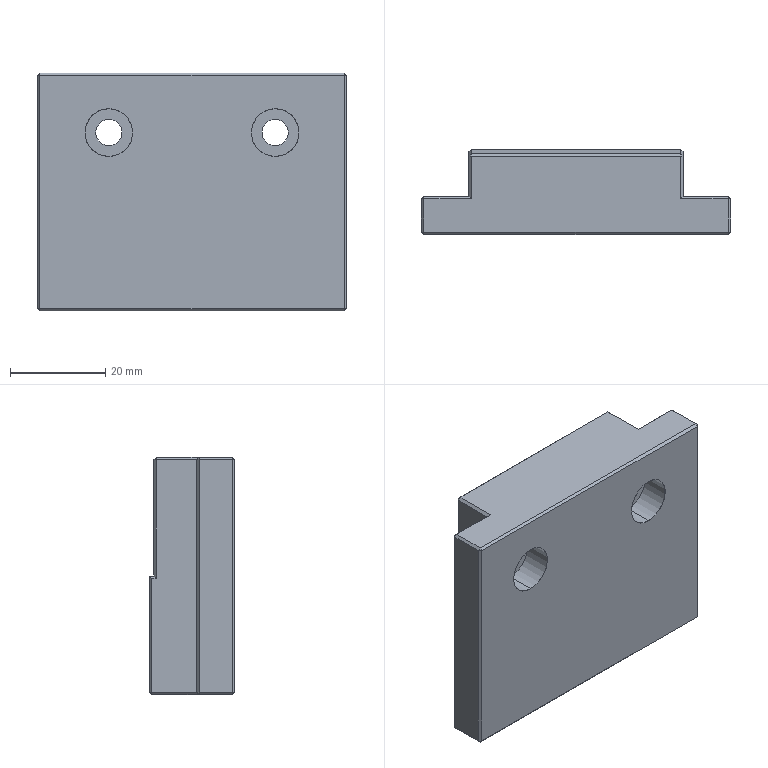Part | SolidWorks | features Chamfer 1, Extrusion 1, HoleWzd 1, ICE 1 | 1 solid | 64 faces | box 65 x 18 x 50 mm | volume 45832 mm3 | plane 52 | cylinder 8 | cone 4 | commonest cylinder face diameters 5.5 x4 10 x4
STEP:
#1=CARTESIAN_POINT('',(50.,0.025,42.5));
#2=VERTEX_POINT('',#1);
#3=CARTESIAN_POINT('',(50.,0.025,32.5));
#4=VERTEX_POINT('',#3);
#5=CARTESIAN_POINT('',(50.,0.025,37.5));
#6=DIRECTION('',(0.,-1.,0.));
#7=DIRECTION('',(0.,0.,-1.));
#8=AXIS2_PLACEMENT_3D('',#5,#6,#7);
#9=CIRCLE('',#8,5.);
#10=EDGE_CURVE('',#2,#4,#9,.T.);
#11=ORIENTED_EDGE('',*,*,#10,.F.);
#12=CARTESIAN_POINT('',(50.,0.,42.525));
#13=VERTEX_POINT('',#12);
#14=CARTESIAN_POINT('',(50.,0.,42.525));
#15=DIRECTION('',(0.,-0.7071,0.7071));
#16=VECTOR('',#15,1000.);
#17=LINE('',#14,#16);
#18=EDGE_CURVE('',#2,#13,#17,.T.);
#19=ORIENTED_EDGE('',*,*,#18,.T.);
#20=CARTESIAN_POINT('',(50.,0.,32.475));
#21=VERTEX_POINT('',#20);
#22=CARTESIAN_POINT('',(50.,0.,37.5));
#23=DIRECTION('',(0.,-1.,0.));
#24=DIRECTION('',(0.,0.,-1.));
#25=AXIS2_PLACEMENT_3D('',#22,#23,#24);
#26=CIRCLE('',#25,5.025);
#27=EDGE_CURVE('',#13,#21,#26,.T.);
#28=ORIENTED_EDGE('',*,*,#27,.T.);
#29=CARTESIAN_POINT('',(50.,0.,32.475));
#30=DIRECTION('',(0.,-0.7071,-0.7071));
#31=VECTOR('',#30,1000.);
#32=LINE('',#29,#31);
#33=EDGE_CURVE('',#4,#21,#32,.T.);
#34=ORIENTED_EDGE('',*,*,#33,.F.);
#35=EDGE_LOOP('',(#11,#19,#28,#34));
#36=FACE_OUTER_BOUND('',#35,.T.);
#37=CARTESIAN_POINT('',(50.,0.,37.5));
#38=DIRECTION('',(0.,-1.,0.));
#39=DIRECTION('',(0.,0.,-1.));
#40=AXIS2_PLACEMENT_3D('',#37,#38,#39);
#41=CONICAL_SURFACE('',#40,5.025,0.7854);
#42=ADVANCED_FACE('',(#36),#41,.F.);
#43=CARTESIAN_POINT('',(50.,6.,42.5));
#44=VERTEX_POINT('',#43);
#45=CARTESIAN_POINT('',(50.,6.,32.5));
#46=VERTEX_POINT('',#45);
#47=CARTESIAN_POINT('',(50.,6.,37.5));
#48=DIRECTION('',(0.,-1.,0.));
#49=DIRECTION('',(0.,0.,-1.));
#50=AXIS2_PLACEMENT_3D('',#47,#48,#49);
#51=CIRCLE('',#50,5.);
#52=EDGE_CURVE('',#44,#46,#51,.T.);
#53=ORIENTED_EDGE('',*,*,#52,.F.);
#54=CARTESIAN_POINT('',(50.,0.,42.5));
#55=DIRECTION('',(0.,-1.,0.));
#56=VECTOR('',#55,1000.);
#57=LINE('',#54,#56);
#58=EDGE_CURVE('',#44,#2,#57,.T.);
#59=ORIENTED_EDGE('',*,*,#58,.T.);
#60=ORIENTED_EDGE('',*,*,#10,.T.);
#61=CARTESIAN_POINT('',(50.,0.,32.5));
#62=DIRECTION('',(0.,-1.,0.));
#63=VECTOR('',#62,1000.);
#64=LINE('',#61,#63);
#65=EDGE_CURVE('',#46,#4,#64,.T.);
#66=ORIENTED_EDGE('',*,*,#65,.F.);
#67=EDGE_LOOP('',(#53,#59,#60,#66));
#68=FACE_OUTER_BOUND('',#67,.T.);
#69=CARTESIAN_POINT('',(50.,0.,37.5));
#70=DIRECTION('',(0.,-1.,0.));
#71=DIRECTION('',(0.,0.,-1.));
#72=AXIS2_PLACEMENT_3D('',#69,#70,#71);
#73=CYLINDRICAL_SURFACE('',#72,5.);
#74=ADVANCED_FACE('',(#68),#73,.F.);
#75=CARTESIAN_POINT('',(50.,17.,34.75));
#76=VERTEX_POINT('',#75);
#77=CARTESIAN_POINT('',(50.,17.,40.25));
#78=VERTEX_POINT('',#77);
#79=CARTESIAN_POINT('',(50.,17.,37.5));
#80=DIRECTION('',(0.,1.,0.));
#81=DIRECTION('',(1.,0.,0.));
#82=AXIS2_PLACEMENT_3D('',#79,#80,#81);
#83=CIRCLE('',#82,2.75);
#84=EDGE_CURVE('',#76,#78,#83,.T.);
#85=ORIENTED_EDGE('',*,*,#84,.T.);
#86=CARTESIAN_POINT('',(50.,6.,40.25));
#87=VERTEX_POINT('',#86);
#88=CARTESIAN_POINT('',(50.,0.,40.25));
#89=DIRECTION('',(0.,-1.,0.));
#90=VECTOR('',#89,1000.);
#91=LINE('',#88,#90);
#92=EDGE_CURVE('',#78,#87,#91,.T.);
#93=ORIENTED_EDGE('',*,*,#92,.T.);
#94=CARTESIAN_POINT('',(50.,6.,34.75));
#95=VERTEX_POINT('',#94);
#96=CARTESIAN_POINT('',(50.,6.,37.5));
#97=DIRECTION('',(0.,-1.,0.));
#98=DIRECTION('',(0.,0.,-1.));
#99=AXIS2_PLACEMENT_3D('',#96,#97,#98);
#100=CIRCLE('',#99,2.75);
#101=EDGE_CURVE('',#87,#95,#100,.T.);
#102=ORIENTED_EDGE('',*,*,#101,.T.);
#103=CARTESIAN_POINT('',(50.,0.,34.75));
#104=DIRECTION('',(0.,-1.,0.));
#105=VECTOR('',#104,1000.);
#106=LINE('',#103,#105);
#107=EDGE_CURVE('',#76,#95,#106,.T.);
#108=ORIENTED_EDGE('',*,*,#107,.F.);
#109=EDGE_LOOP('',(#85,#93,#102,#108));
#110=FACE_OUTER_BOUND('',#109,.T.);
#111=CARTESIAN_POINT('',(50.,0.,37.5));
#112=DIRECTION('',(0.,-1.,0.));
#113=DIRECTION('',(0.,0.,-1.));
#114=AXIS2_PLACEMENT_3D('',#111,#112,#113);
#115=CYLINDRICAL_SURFACE('',#114,2.75);
#116=ADVANCED_FACE('',(#110),#115,.F.);
#117=CARTESIAN_POINT('',(15.,0.025,42.5));
#118=VERTEX_POINT('',#117);
#119=CARTESIAN_POINT('',(15.,0.025,32.5));
#120=VERTEX_POINT('',#119);
#121=CARTESIAN_POINT('',(15.,0.025,37.5));
#122=DIRECTION('',(0.,-1.,0.));
#123=DIRECTION('',(0.,0.,-1.));
#124=AXIS2_PLACEMENT_3D('',#121,#122,#123);
#125=CIRCLE('',#124,5.);
#126=EDGE_CURVE('',#118,#120,#125,.T.);
#127=ORIENTED_EDGE('',*,*,#126,.F.);
#128=CARTESIAN_POINT('',(15.,0.,42.525));
#129=VERTEX_POINT('',#128);
#130=CARTESIAN_POINT('',(15.,0.,42.525));
#131=DIRECTION('',(0.,-0.7071,0.7071));
#132=VECTOR('',#131,1000.);
#133=LINE('',#130,#132);
#134=EDGE_CURVE('',#118,#129,#133,.T.);
#135=ORIENTED_EDGE('',*,*,#134,.T.);
#136=CARTESIAN_POINT('',(15.,0.,32.475));
#137=VERTEX_POINT('',#136);
#138=CARTESIAN_POINT('',(15.,0.,37.5));
#139=DIRECTION('',(0.,-1.,0.));
#140=DIRECTION('',(0.,0.,-1.));
#141=AXIS2_PLACEMENT_3D('',#138,#139,#140);
#142=CIRCLE('',#141,5.025);
#143=EDGE_CURVE('',#129,#137,#142,.T.);
#144=ORIENTED_EDGE('',*,*,#143,.T.);
#145=CARTESIAN_POINT('',(15.,0.,32.475));
#146=DIRECTION('',(0.,-0.7071,-0.7071));
#147=VECTOR('',#146,1000.);
#148=LINE('',#145,#147);
#149=EDGE_CURVE('',#120,#137,#148,.T.);
#150=ORIENTED_EDGE('',*,*,#149,.F.);
#151=EDGE_LOOP('',(#127,#135,#144,#150));
#152=FACE_OUTER_BOUND('',#151,.T.);
#153=CARTESIAN_POINT('',(15.,0.,37.5));
#154=DIRECTION('',(0.,-1.,0.));
#155=DIRECTION('',(0.,0.,-1.));
#156=AXIS2_PLACEMENT_3D('',#153,#154,#155);
#157=CONICAL_SURFACE('',#156,5.025,0.7854);
#158=ADVANCED_FACE('',(#152),#157,.F.);
#159=CARTESIAN_POINT('',(15.,6.,42.5));
#160=VERTEX_POINT('',#159);
#161=CARTESIAN_POINT('',(15.,6.,32.5));
#162=VERTEX_POINT('',#161);
#163=CARTESIAN_POINT('',(15.,6.,37.5));
#164=DIRECTION('',(0.,-1.,0.));
#165=DIRECTION('',(0.,0.,-1.));
#166=AXIS2_PLACEMENT_3D('',#163,#164,#165);
#167=CIRCLE('',#166,5.);
#168=EDGE_CURVE('',#160,#162,#167,.T.);
#169=ORIENTED_EDGE('',*,*,#168,.F.);
#170=CARTESIAN_POINT('',(15.,0.,42.5));
#171=DIRECTION('',(0.,-1.,0.));
#172=VECTOR('',#171,1000.);
#173=LINE('',#170,#172);
#174=EDGE_CURVE('',#160,#118,#173,.T.);
#175=ORIENTED_EDGE('',*,*,#174,.T.);
#176=ORIENTED_EDGE('',*,*,#126,.T.);
#177=CARTESIAN_POINT('',(15.,0.,32.5));
#178=DIRECTION('',(0.,-1.,0.));
#179=VECTOR('',#178,1000.);
#180=LINE('',#177,#179);
#181=EDGE_CURVE('',#162,#120,#180,.T.);
#182=ORIENTED_EDGE('',*,*,#181,.F.);
#183=EDGE_LOOP('',(#169,#175,#176,#182));
#184=FACE_OUTER_BOUND('',#183,.T.);
#185=CARTESIAN_POINT('',(15.,0.,37.5));
#186=DIRECTION('',(0.,-1.,0.));
#187=DIRECTION('',(0.,0.,-1.));
#188=AXIS2_PLACEMENT_3D('',#185,#186,#187);
#189=CYLINDRICAL_SURFACE('',#188,5.);
#190=ADVANCED_FACE('',(#184),#189,.F.);
#191=CARTESIAN_POINT('',(15.,17.,34.75));
#192=VERTEX_POINT('',#191);
#193=CARTESIAN_POINT('',(15.,17.,40.25));
#194=VERTEX_POINT('',#193);
#195=CARTESIAN_POINT('',(15.,17.,37.5));
#196=DIRECTION('',(0.,1.,0.));
#197=DIRECTION('',(1.,0.,0.));
#198=AXIS2_PLACEMENT_3D('',#195,#196,#197);
#199=CIRCLE('',#198,2.75);
#200=EDGE_CURVE('',#192,#194,#199,.T.);
#201=ORIENTED_EDGE('',*,*,#200,.T.);
#202=CARTESIAN_POINT('',(15.,6.,40.25));
#203=VERTEX_POINT('',#202);
#204=CARTESIAN_POINT('',(15.,0.,40.25));
#205=DIRECTION('',(0.,-1.,0.));
#206=VECTOR('',#205,1000.);
#207=LINE('',#204,#206);
#208=EDGE_CURVE('',#194,#203,#207,.T.);
#209=ORIENTED_EDGE('',*,*,#208,.T.);
#210=CARTESIAN_POINT('',(15.,6.,34.75));
#211=VERTEX_POINT('',#210);
#212=CARTESIAN_POINT('',(15.,6.,37.5));
#213=DIRECTION('',(0.,-1.,0.));
#214=DIRECTION('',(0.,0.,-1.));
#215=AXIS2_PLACEMENT_3D('',#212,#213,#214);
#216=CIRCLE('',#215,2.75);
#217=EDGE_CURVE('',#203,#211,#216,.T.);
#218=ORIENTED_EDGE('',*,*,#217,.T.);
#219=CARTESIAN_POINT('',(15.,0.,34.75));
#220=DIRECTION('',(0.,-1.,0.));
#221=VECTOR('',#220,1000.);
#222=LINE('',#219,#221);
#223=EDGE_CURVE('',#192,#211,#222,.T.);
#224=ORIENTED_EDGE('',*,*,#223,.F.);
#225=EDGE_LOOP('',(#201,#209,#218,#224));
#226=FACE_OUTER_BOUND('',#225,.T.);
#227=CARTESIAN_POINT('',(15.,0.,37.5));
#228=DIRECTION('',(0.,-1.,0.));
#229=DIRECTION('',(0.,0.,-1.));
#230=AXIS2_PLACEMENT_3D('',#227,#228,#229);
#231=CYLINDRICAL_SURFACE('',#230,2.75);
#232=ADVANCED_FACE('',(#226),#231,.F.);
#233=CARTESIAN_POINT('',(0.,7.5,49.5));
#234=VERTEX_POINT('',#233);
#235=CARTESIAN_POINT('',(0.,7.5,0.5));
#236=VERTEX_POINT('',#235);
#237=CARTESIAN_POINT('',(0.,7.5,50.));
#238=DIRECTION('',(0.,0.,-1.));
#239=VECTOR('',#238,1000.);
#240=LINE('',#237,#239);
#241=EDGE_CURVE('',#234,#236,#240,.T.);
#242=ORIENTED_EDGE('',*,*,#241,.T.);
#243=CARTESIAN_POINT('',(0.,0.5,0.5));
#244=VERTEX_POINT('',#243);
#245=CARTESIAN_POINT('',(0.,0.,0.5));
#246=DIRECTION('',(0.,-1.,0.));
#247=VECTOR('',#246,1000.);
#248=LINE('',#245,#247);
#249=EDGE_CURVE('',#236,#244,#248,.T.);
#250=ORIENTED_EDGE('',*,*,#249,.T.);
#251=CARTESIAN_POINT('',(0.,0.5,49.5));
#252=VERTEX_POINT('',#251);
#253=CARTESIAN_POINT('',(0.,0.5,50.));
#254=DIRECTION('',(0.,0.,1.));
#255=VECTOR('',#254,1000.);
#256=LINE('',#253,#255);
#257=EDGE_CURVE('',#244,#252,#256,.T.);
#258=ORIENTED_EDGE('',*,*,#257,.T.);
#259=CARTESIAN_POINT('',(0.,0.,49.5));
#260=DIRECTION('',(0.,1.,0.));
#261=VECTOR('',#260,1000.);
#262=LINE('',#259,#261);
#263=EDGE_CURVE('',#252,#234,#262,.T.);
#264=ORIENTED_EDGE('',*,*,#263,.T.);
#265=EDGE_LOOP('',(#242,#250,#258,#264));
#266=FACE_OUTER_BOUND('',#265,.T.);
#267=CARTESIAN_POINT('',(0.,0.,50.));
#268=DIRECTION('',(1.,0.,0.));
#269=DIRECTION('',(0.,0.,-1.));
#270=AXIS2_PLACEMENT_3D('',#267,#268,#269);
#271=PLANE('',#270);
#272=ADVANCED_FACE('',(#266),#271,.F.);
#273=CARTESIAN_POINT('',(0.5,0.,49.5));
#274=VERTEX_POINT('',#273);
#275=CARTESIAN_POINT('',(0.5,0.,0.5));
#276=VERTEX_POINT('',#275);
#277=CARTESIAN_POINT('',(0.5,0.,50.));
#278=DIRECTION('',(0.,0.,-1.));
#279=VECTOR('',#278,1000.);
#280=LINE('',#277,#279);
#281=EDGE_CURVE('',#274,#276,#280,.T.);
#282=ORIENTED_EDGE('',*,*,#281,.T.);
#283=CARTESIAN_POINT('',(64.5,0.,0.5));
#284=VERTEX_POINT('',#283);
#285=CARTESIAN_POINT('',(65.,0.,0.5));
#286=DIRECTION('',(1.,0.,0.));
#287=VECTOR('',#286,1000.);
#288=LINE('',#285,#287);
#289=EDGE_CURVE('',#276,#284,#288,.T.);
#290=ORIENTED_EDGE('',*,*,#289,.T.);
#291=CARTESIAN_POINT('',(64.5,0.,49.5));
#292=VERTEX_POINT('',#291);
#293=CARTESIAN_POINT('',(64.5,0.,50.));
#294=DIRECTION('',(0.,0.,1.));
#295=VECTOR('',#294,1000.);
#296=LINE('',#293,#295);
#297=EDGE_CURVE('',#284,#292,#296,.T.);
#298=ORIENTED_EDGE('',*,*,#297,.T.);
#299=CARTESIAN_POINT('',(0.,0.,49.5));
#300=DIRECTION('',(-1.,0.,0.));
#301=VECTOR('',#300,1000.);
#302=LINE('',#299,#301);
#303=EDGE_CURVE('',#292,#274,#302,.T.);
#304=ORIENTED_EDGE('',*,*,#303,.T.);
#305=EDGE_LOOP('',(#282,#290,#298,#304));
#306=FACE_OUTER_BOUND('',#305,.T.);
#307=CARTESIAN_POINT('',(50.,0.,37.5));
#308=DIRECTION('',(0.,-1.,0.));
#309=DIRECTION('',(0.,0.,-1.));
#310=AXIS2_PLACEMENT_3D('',#307,#308,#309);
#311=CIRCLE('',#310,5.025);
#312=EDGE_CURVE('',#21,#13,#311,.T.);
#313=ORIENTED_EDGE('',*,*,#312,.F.);
#314=ORIENTED_EDGE('',*,*,#27,.F.);
#315=EDGE_LOOP('',(#313,#314));
#316=FACE_BOUND('',#315,.T.);
#317=CARTESIAN_POINT('',(15.,0.,37.5));
#318=DIRECTION('',(0.,-1.,0.));
#319=DIRECTION('',(0.,0.,-1.));
#320=AXIS2_PLACEMENT_3D('',#317,#318,#319);
#321=CIRCLE('',#320,5.025);
#322=EDGE_CURVE('',#137,#129,#321,.T.);
#323=ORIENTED_EDGE('',*,*,#322,.F.);
#324=ORIENTED_EDGE('',*,*,#143,.F.);
#325=EDGE_LOOP('',(#323,#324));
#326=FACE_BOUND('',#325,.T.);
#327=CARTESIAN_POINT('',(0.,0.,50.));
#328=DIRECTION('',(0.,1.,0.));
#329=DIRECTION('',(0.,0.,1.));
#330=AXIS2_PLACEMENT_3D('',#327,#328,#329);
#331=PLANE('',#330);
#332=ADVANCED_FACE('',(#306,#316,#326),#331,.F.);
#333=CARTESIAN_POINT('',(65.,0.5,49.5));
#334=VERTEX_POINT('',#333);
#335=CARTESIAN_POINT('',(65.,0.5,0.5));
#336=VERTEX_POINT('',#335);
#337=CARTESIAN_POINT('',(65.,0.5,50.));
#338=DIRECTION('',(0.,0.,-1.));
#339=VECTOR('',#338,1000.);
#340=LINE('',#337,#339);
#341=EDGE_CURVE('',#334,#336,#340,.T.);
#342=ORIENTED_EDGE('',*,*,#341,.T.);
#343=CARTESIAN_POINT('',(65.,7.5,0.5));
#344=VERTEX_POINT('',#343);
#345=CARTESIAN_POINT('',(65.,8.,0.5));
#346=DIRECTION('',(0.,1.,0.));
#347=VECTOR('',#346,1000.);
#348=LINE('',#345,#347);
#349=EDGE_CURVE('',#336,#344,#348,.T.);
#350=ORIENTED_EDGE('',*,*,#349,.T.);
#351=CARTESIAN_POINT('',(65.,7.5,49.5));
#352=VERTEX_POINT('',#351);
#353=CARTESIAN_POINT('',(65.,7.5,50.));
#354=DIRECTION('',(0.,0.,1.));
#355=VECTOR('',#354,1000.);
#356=LINE('',#353,#355);
#357=EDGE_CURVE('',#344,#352,#356,.T.);
#358=ORIENTED_EDGE('',*,*,#357,.T.);
#359=CARTESIAN_POINT('',(65.,0.,49.5));
#360=DIRECTION('',(0.,-1.,0.));
#361=VECTOR('',#360,1000.);
#362=LINE('',#359,#361);
#363=EDGE_CURVE('',#352,#334,#362,.T.);
#364=ORIENTED_EDGE('',*,*,#363,.T.);
#365=EDGE_LOOP('',(#342,#350,#358,#364));
#366=FACE_OUTER_BOUND('',#365,.T.);
#367=CARTESIAN_POINT('',(65.,0.,50.));
#368=DIRECTION('',(-1.,0.,0.));
#369=DIRECTION('',(0.,0.,1.));
#370=AXIS2_PLACEMENT_3D('',#367,#368,#369);
#371=PLANE('',#370);
#372=ADVANCED_FACE('',(#366),#371,.F.);
#373=CARTESIAN_POINT('',(64.5,8.,49.5));
#374=VERTEX_POINT('',#373);
#375=CARTESIAN_POINT('',(64.5,8.,0.5));
#376=VERTEX_POINT('',#375);
#377=CARTESIAN_POINT('',(64.5,8.,50.));
#378=DIRECTION('',(0.,0.,-1.));
#379=VECTOR('',#378,1000.);
#380=LINE('',#377,#379);
#381=EDGE_CURVE('',#374,#376,#380,.T.);
#382=ORIENTED_EDGE('',*,*,#381,.T.);
#383=CARTESIAN_POINT('',(55.,8.,0.5));
#384=VERTEX_POINT('',#383);
#385=CARTESIAN_POINT('',(55.,8.,0.5));
#386=DIRECTION('',(-1.,0.,0.));
#387=VECTOR('',#386,1000.);
#388=LINE('',#385,#387);
#389=EDGE_CURVE('',#376,#384,#388,.T.);
#390=ORIENTED_EDGE('',*,*,#389,.T.);
#391=CARTESIAN_POINT('',(55.,8.,49.5));
#392=VERTEX_POINT('',#391);
#393=CARTESIAN_POINT('',(55.,8.,50.));
#394=DIRECTION('',(0.,0.,-1.));
#395=VECTOR('',#394,1000.);
#396=LINE('',#393,#395);
#397=EDGE_CURVE('',#392,#384,#396,.T.);
#398=ORIENTED_EDGE('',*,*,#397,.F.);
#399=CARTESIAN_POINT('',(55.,8.,49.5));
#400=DIRECTION('',(1.,0.,0.));
#401=VECTOR('',#400,1000.);
#402=LINE('',#399,#401);
#403=EDGE_CURVE('',#392,#374,#402,.T.);
#404=ORIENTED_EDGE('',*,*,#403,.T.);
#405=EDGE_LOOP('',(#382,#390,#398,#404));
#406=FACE_OUTER_BOUND('',#405,.T.);
#407=CARTESIAN_POINT('',(55.,8.,50.));
#408=DIRECTION('',(0.,-1.,0.));
#409=DIRECTION('',(1.,0.,0.));
#410=AXIS2_PLACEMENT_3D('',#407,#408,#409);
#411=PLANE('',#410);
#412=ADVANCED_FACE('',(#406),#411,.F.);
#413=ORIENTED_EDGE('',*,*,#397,.T.);
#414=CARTESIAN_POINT('',(55.,17.5,0.5));
#415=VERTEX_POINT('',#414);
#416=CARTESIAN_POINT('',(55.,18.,0.5));
#417=DIRECTION('',(0.,1.,0.));
#418=VECTOR('',#417,1000.);
#419=LINE('',#416,#418);
#420=EDGE_CURVE('',#384,#415,#419,.T.);
#421=ORIENTED_EDGE('',*,*,#420,.T.);
#422=CARTESIAN_POINT('',(55.,17.5,24.5));
#423=VERTEX_POINT('',#422);
#424=CARTESIAN_POINT('',(55.,17.5,50.));
#425=DIRECTION('',(0.,0.,1.));
#426=VECTOR('',#425,1000.);
#427=LINE('',#424,#426);
#428=EDGE_CURVE('',#415,#423,#427,.T.);
#429=ORIENTED_EDGE('',*,*,#428,.T.);
#430=CARTESIAN_POINT('',(55.,16.5,24.5));
#431=VERTEX_POINT('',#430);
#432=CARTESIAN_POINT('',(55.,18.,24.5));
#433=DIRECTION('',(0.,-1.,0.));
#434=VECTOR('',#433,1000.);
#435=LINE('',#432,#434);
#436=EDGE_CURVE('',#423,#431,#435,.T.);
#437=ORIENTED_EDGE('',*,*,#436,.T.);
#438=CARTESIAN_POINT('',(55.,16.5,49.5));
#439=VERTEX_POINT('',#438);
#440=CARTESIAN_POINT('',(55.,16.5,50.));
#441=DIRECTION('',(0.,0.,1.));
#442=VECTOR('',#441,1000.);
#443=LINE('',#440,#442);
#444=EDGE_CURVE('',#431,#439,#443,.T.);
#445=ORIENTED_EDGE('',*,*,#444,.T.);
#446=CARTESIAN_POINT('',(55.,18.,49.5));
#447=DIRECTION('',(0.,-1.,0.));
#448=VECTOR('',#447,1000.);
#449=LINE('',#446,#448);
#450=EDGE_CURVE('',#439,#392,#449,.T.);
#451=ORIENTED_EDGE('',*,*,#450,.T.);
#452=EDGE_LOOP('',(#413,#421,#429,#437,#445,#451));
#453=FACE_OUTER_BOUND('',#452,.T.);
#454=CARTESIAN_POINT('',(55.,18.,50.));
#455=DIRECTION('',(-1.,0.,0.));
#456=DIRECTION('',(0.,-1.,0.));
#457=AXIS2_PLACEMENT_3D('',#454,#455,#456);
#458=PLANE('',#457);
#459=ADVANCED_FACE('',(#453),#458,.F.);
#460=CARTESIAN_POINT('',(54.5,18.,0.5));
#461=VERTEX_POINT('',#460);
#462=CARTESIAN_POINT('',(10.5,18.,0.5));
#463=VERTEX_POINT('',#462);
#464=CARTESIAN_POINT('',(10.,18.,0.5));
#465=DIRECTION('',(-1.,0.,0.));
#466=VECTOR('',#465,1000.);
#467=LINE('',#464,#466);
#468=EDGE_CURVE('',#461,#463,#467,.T.);
#469=ORIENTED_EDGE('',*,*,#468,.T.);
#470=CARTESIAN_POINT('',(10.5,18.,25.));
#471=VERTEX_POINT('',#470);
#472=CARTESIAN_POINT('',(10.5,18.,50.));
#473=DIRECTION('',(0.,0.,1.));
#474=VECTOR('',#473,1000.);
#475=LINE('',#472,#474);
#476=EDGE_CURVE('',#463,#471,#475,.T.);
#477=ORIENTED_EDGE('',*,*,#476,.T.);
#478=CARTESIAN_POINT('',(54.5,18.,25.));
#479=VERTEX_POINT('',#478);
#480=CARTESIAN_POINT('',(10.,18.,25.));
#481=DIRECTION('',(-1.,0.,0.));
#482=VECTOR('',#481,1000.);
#483=LINE('',#480,#482);
#484=EDGE_CURVE('',#479,#471,#483,.T.);
#485=ORIENTED_EDGE('',*,*,#484,.F.);
#486=CARTESIAN_POINT('',(54.5,18.,50.));
#487=DIRECTION('',(0.,0.,-1.));
#488=VECTOR('',#487,1000.);
#489=LINE('',#486,#488);
#490=EDGE_CURVE('',#479,#461,#489,.T.);
#491=ORIENTED_EDGE('',*,*,#490,.T.);
#492=EDGE_LOOP('',(#469,#477,#485,#491));
#493=FACE_OUTER_BOUND('',#492,.T.);
#494=CARTESIAN_POINT('',(10.,18.,50.));
#495=DIRECTION('',(0.,-1.,0.));
#496=DIRECTION('',(1.,0.,0.));
#497=AXIS2_PLACEMENT_3D('',#494,#495,#496);
#498=PLANE('',#497);
#499=ADVANCED_FACE('',(#493),#498,.F.);
#500=CARTESIAN_POINT('',(10.,17.5,24.5));
#501=VERTEX_POINT('',#500);
#502=CARTESIAN_POINT('',(10.,17.5,0.5));
#503=VERTEX_POINT('',#502);
#504=CARTESIAN_POINT('',(10.,17.5,50.));
#505=DIRECTION('',(0.,0.,-1.));
#506=VECTOR('',#505,1000.);
#507=LINE('',#504,#506);
#508=EDGE_CURVE('',#501,#503,#507,.T.);
#509=ORIENTED_EDGE('',*,*,#508,.T.);
#510=CARTESIAN_POINT('',(10.,8.,0.5));
#511=VERTEX_POINT('',#510);
#512=CARTESIAN_POINT('',(10.,8.,0.5));
#513=DIRECTION('',(0.,-1.,0.));
#514=VECTOR('',#513,1000.);
#515=LINE('',#512,#514);
#516=EDGE_CURVE('',#503,#511,#515,.T.);
#517=ORIENTED_EDGE('',*,*,#516,.T.);
#518=CARTESIAN_POINT('',(10.,8.,49.5));
#519=VERTEX_POINT('',#518);
#520=CARTESIAN_POINT('',(10.,8.,50.));
#521=DIRECTION('',(0.,0.,-1.));
#522=VECTOR('',#521,1000.);
#523=LINE('',#520,#522);
#524=EDGE_CURVE('',#519,#511,#523,.T.);
#525=ORIENTED_EDGE('',*,*,#524,.F.);
#526=CARTESIAN_POINT('',(10.,16.5,49.5));
#527=VERTEX_POINT('',#526);
#528=CARTESIAN_POINT('',(10.,18.,49.5));
#529=DIRECTION('',(0.,1.,0.));
#530=VECTOR('',#529,1000.);
#531=LINE('',#528,#530);
#532=EDGE_CURVE('',#519,#527,#531,.T.);
#533=ORIENTED_EDGE('',*,*,#532,.T.);
#534=CARTESIAN_POINT('',(10.,16.5,24.5));
#535=VERTEX_POINT('',#534);
#536=CARTESIAN_POINT('',(10.,16.5,50.));
#537=DIRECTION('',(0.,0.,-1.));
#538=VECTOR('',#537,1000.);
#539=LINE('',#536,#538);
#540=EDGE_CURVE('',#527,#535,#539,.T.);
#541=ORIENTED_EDGE('',*,*,#540,.T.);
#542=CARTESIAN_POINT('',(10.,18.,24.5));
#543=DIRECTION('',(0.,1.,0.));
#544=VECTOR('',#543,1000.);
#545=LINE('',#542,#544);
#546=EDGE_CURVE('',#535,#501,#545,.T.);
#547=ORIENTED_EDGE('',*,*,#546,.T.);
#548=EDGE_LOOP('',(#509,#517,#525,#533,#541,#547));
#549=FACE_OUTER_BOUND('',#548,.T.);
#550=CARTESIAN_POINT('',(10.,18.,50.));
#551=DIRECTION('',(1.,0.,0.));
#552=DIRECTION('',(0.,1.,0.));
#553=AXIS2_PLACEMENT_3D('',#550,#551,#552);
#554=PLANE('',#553);
#555=ADVANCED_FACE('',(#549),#554,.F.);
#556=ORIENTED_EDGE('',*,*,#524,.T.);
#557=CARTESIAN_POINT('',(0.5,8.,0.5));
#558=VERTEX_POINT('',#557);
#559=CARTESIAN_POINT('',(0.,8.,0.5));
#560=DIRECTION('',(-1.,0.,0.));
#561=VECTOR('',#560,1000.);
#562=LINE('',#559,#561);
#563=EDGE_CURVE('',#511,#558,#562,.T.);
#564=ORIENTED_EDGE('',*,*,#563,.T.);
#565=CARTESIAN_POINT('',(0.5,8.,49.5));
#566=VERTEX_POINT('',#565);
#567=CARTESIAN_POINT('',(0.5,8.,50.));
#568=DIRECTION('',(0.,0.,1.));
#569=VECTOR('',#568,1000.);
#570=LINE('',#567,#569);
#571=EDGE_CURVE('',#558,#566,#570,.T.);
#572=ORIENTED_EDGE('',*,*,#571,.T.);
#573=CARTESIAN_POINT('',(0.,8.,49.5));
#574=DIRECTION('',(1.,0.,0.));
#575=VECTOR('',#574,1000.);
#576=LINE('',#573,#575);
#577=EDGE_CURVE('',#566,#519,#576,.T.);
#578=ORIENTED_EDGE('',*,*,#577,.T.);
#579=EDGE_LOOP('',(#556,#564,#572,#578));
#580=FACE_OUTER_BOUND('',#579,.T.);
#581=CARTESIAN_POINT('',(0.,8.,50.));
#582=DIRECTION('',(0.,-1.,0.));
#583=DIRECTION('',(0.,0.,-1.));
#584=AXIS2_PLACEMENT_3D('',#581,#582,#583);
#585=PLANE('',#584);
#586=ADVANCED_FACE('',(#580),#585,.F.);
#587=CARTESIAN_POINT('',(64.5,0.5,50.));
#588=VERTEX_POINT('',#587);
#589=CARTESIAN_POINT('',(64.5,7.5,50.));
#590=VERTEX_POINT('',#589);
#591=CARTESIAN_POINT('',(64.5,0.,50.));
#592=DIRECTION('',(0.,1.,0.));
#593=VECTOR('',#592,1000.);
#594=LINE('',#591,#593);
#595=EDGE_CURVE('',#588,#590,#594,.T.);
#596=ORIENTED_EDGE('',*,*,#595,.T.);
#597=CARTESIAN_POINT('',(54.5,7.5,50.));
#598=VERTEX_POINT('',#597);
#599=CARTESIAN_POINT('',(0.,7.5,50.));
#600=DIRECTION('',(-1.,0.,0.));
#601=VECTOR('',#600,1000.);
#602=LINE('',#599,#601);
#603=EDGE_CURVE('',#590,#598,#602,.T.);
#604=ORIENTED_EDGE('',*,*,#603,.T.);
#605=CARTESIAN_POINT('',(54.5,16.5,50.));
#606=VERTEX_POINT('',#605);
#607=CARTESIAN_POINT('',(54.5,0.,50.));
#608=DIRECTION('',(0.,1.,0.));
#609=VECTOR('',#608,1000.);
#610=LINE('',#607,#609);
#611=EDGE_CURVE('',#598,#606,#610,.T.);
#612=ORIENTED_EDGE('',*,*,#611,.T.);
#613=CARTESIAN_POINT('',(10.5,16.5,50.));
#614=VERTEX_POINT('',#613);
#615=CARTESIAN_POINT('',(0.,16.5,50.));
#616=DIRECTION('',(-1.,0.,0.));
#617=VECTOR('',#616,1000.);
#618=LINE('',#615,#617);
#619=EDGE_CURVE('',#606,#614,#618,.T.);
#620=ORIENTED_EDGE('',*,*,#619,.T.);
#621=CARTESIAN_POINT('',(10.5,7.5,50.));
#622=VERTEX_POINT('',#621);
#623=CARTESIAN_POINT('',(10.5,0.,50.));
#624=DIRECTION('',(0.,-1.,0.));
#625=VECTOR('',#624,1000.);
#626=LINE('',#623,#625);
#627=EDGE_CURVE('',#614,#622,#626,.T.);
#628=ORIENTED_EDGE('',*,*,#627,.T.);
#629=CARTESIAN_POINT('',(0.5,7.5,50.));
#630=VERTEX_POINT('',#629);
#631=CARTESIAN_POINT('',(0.,7.5,50.));
#632=DIRECTION('',(-1.,0.,0.));
#633=VECTOR('',#632,1000.);
#634=LINE('',#631,#633);
#635=EDGE_CURVE('',#622,#630,#634,.T.);
#636=ORIENTED_EDGE('',*,*,#635,.T.);
#637=CARTESIAN_POINT('',(0.5,0.5,50.));
#638=VERTEX_POINT('',#637);
#639=CARTESIAN_POINT('',(0.5,0.,50.));
#640=DIRECTION('',(0.,-1.,0.));
#641=VECTOR('',#640,1000.);
#642=LINE('',#639,#641);
#643=EDGE_CURVE('',#630,#638,#642,.T.);
#644=ORIENTED_EDGE('',*,*,#643,.T.);
#645=CARTESIAN_POINT('',(0.,0.5,50.));
#646=DIRECTION('',(1.,0.,0.));
#647=VECTOR('',#646,1000.);
#648=LINE('',#645,#647);
#649=EDGE_CURVE('',#638,#588,#648,.T.);
#650=ORIENTED_EDGE('',*,*,#649,.T.);
#651=EDGE_LOOP('',(#596,#604,#612,#620,#628,#636,#644,#650));
#652=FACE_OUTER_BOUND('',#651,.T.);
#653=CARTESIAN_POINT('',(0.,0.,50.));
#654=DIRECTION('',(0.,0.,-1.));
#655=DIRECTION('',(-1.,0.,0.));
#656=AXIS2_PLACEMENT_3D('',#653,#654,#655);
#657=PLANE('',#656);
#658=ADVANCED_FACE('',(#652),#657,.F.);
#659=CARTESIAN_POINT('',(64.5,7.5,0.));
#660=VERTEX_POINT('',#659);
#661=CARTESIAN_POINT('',(64.5,0.5,0.));
#662=VERTEX_POINT('',#661);
#663=CARTESIAN_POINT('',(64.5,0.,0.));
#664=DIRECTION('',(0.,-1.,0.));
#665=VECTOR('',#664,1000.);
#666=LINE('',#663,#665);
#667=EDGE_CURVE('',#660,#662,#666,.T.);
#668=ORIENTED_EDGE('',*,*,#667,.T.);
#669=CARTESIAN_POINT('',(0.5,0.5,0.));
#670=VERTEX_POINT('',#669);
#671=CARTESIAN_POINT('',(0.,0.5,0.));
#672=DIRECTION('',(-1.,0.,0.));
#673=VECTOR('',#672,1000.);
#674=LINE('',#671,#673);
#675=EDGE_CURVE('',#662,#670,#674,.T.);
#676=ORIENTED_EDGE('',*,*,#675,.T.);
#677=CARTESIAN_POINT('',(0.5,7.5,0.));
#678=VERTEX_POINT('',#677);
#679=CARTESIAN_POINT('',(0.5,8.,0.));
#680=DIRECTION('',(0.,1.,0.));
#681=VECTOR('',#680,1000.);
#682=LINE('',#679,#681);
#683=EDGE_CURVE('',#670,#678,#682,.T.);
#684=ORIENTED_EDGE('',*,*,#683,.T.);
#685=CARTESIAN_POINT('',(10.5,7.5,0.));
#686=VERTEX_POINT('',#685);
#687=CARTESIAN_POINT('',(10.,7.5,0.));
#688=DIRECTION('',(1.,0.,0.));
#689=VECTOR('',#688,1000.);
#690=LINE('',#687,#689);
#691=EDGE_CURVE('',#678,#686,#690,.T.);
#692=ORIENTED_EDGE('',*,*,#691,.T.);
#693=CARTESIAN_POINT('',(10.5,17.5,0.));
#694=VERTEX_POINT('',#693);
#695=CARTESIAN_POINT('',(10.5,18.,0.));
#696=DIRECTION('',(0.,1.,0.));
#697=VECTOR('',#696,1000.);
#698=LINE('',#695,#697);
#699=EDGE_CURVE('',#686,#694,#698,.T.);
#700=ORIENTED_EDGE('',*,*,#699,.T.);
#701=CARTESIAN_POINT('',(54.5,17.5,0.));
#702=VERTEX_POINT('',#701);
#703=CARTESIAN_POINT('',(55.,17.5,0.));
#704=DIRECTION('',(1.,0.,0.));
#705=VECTOR('',#704,1000.);
#706=LINE('',#703,#705);
#707=EDGE_CURVE('',#694,#702,#706,.T.);
#708=ORIENTED_EDGE('',*,*,#707,.T.);
#709=CARTESIAN_POINT('',(54.5,7.5,0.));
#710=VERTEX_POINT('',#709);
#711=CARTESIAN_POINT('',(54.5,8.,0.));
#712=DIRECTION('',(0.,-1.,0.));
#713=VECTOR('',#712,1000.);
#714=LINE('',#711,#713);
#715=EDGE_CURVE('',#702,#710,#714,.T.);
#716=ORIENTED_EDGE('',*,*,#715,.T.);
#717=CARTESIAN_POINT('',(65.,7.5,0.));
#718=DIRECTION('',(1.,0.,0.));
#719=VECTOR('',#718,1000.);
#720=LINE('',#717,#719);
#721=EDGE_CURVE('',#710,#660,#720,.T.);
#722=ORIENTED_EDGE('',*,*,#721,.T.);
#723=EDGE_LOOP('',(#668,#676,#684,#692,#700,#708,#716,#722));
#724=FACE_OUTER_BOUND('',#723,.T.);
#725=CARTESIAN_POINT('',(0.,0.,0.));
#726=DIRECTION('',(0.,0.,-1.));
#727=DIRECTION('',(-1.,0.,0.));
#728=AXIS2_PLACEMENT_3D('',#725,#726,#727);
#729=PLANE('',#728);
#730=ADVANCED_FACE('',(#724),#729,.T.);
#731=ORIENTED_EDGE('',*,*,#208,.F.);
#732=CARTESIAN_POINT('',(15.,17.,37.5));
#733=DIRECTION('',(0.,1.,0.));
#734=DIRECTION('',(1.,0.,0.));
#735=AXIS2_PLACEMENT_3D('',#732,#733,#734);
#736=CIRCLE('',#735,2.75);
#737=EDGE_CURVE('',#194,#192,#736,.T.);
#738=ORIENTED_EDGE('',*,*,#737,.T.);
#739=ORIENTED_EDGE('',*,*,#223,.T.);
#740=CARTESIAN_POINT('',(15.,6.,37.5));
#741=DIRECTION('',(0.,-1.,0.));
#742=DIRECTION('',(0.,0.,-1.));
#743=AXIS2_PLACEMENT_3D('',#740,#741,#742);
#744=CIRCLE('',#743,2.75);
#745=EDGE_CURVE('',#211,#203,#744,.T.);
#746=ORIENTED_EDGE('',*,*,#745,.T.);
#747=EDGE_LOOP('',(#731,#738,#739,#746));
#748=FACE_OUTER_BOUND('',#747,.T.);
#749=CARTESIAN_POINT('',(15.,0.,37.5));
#750=DIRECTION('',(0.,-1.,0.));
#751=DIRECTION('',(0.,0.,-1.));
#752=AXIS2_PLACEMENT_3D('',#749,#750,#751);
#753=CYLINDRICAL_SURFACE('',#752,2.75);
#754=ADVANCED_FACE('',(#748),#753,.F.);
#755=ORIENTED_EDGE('',*,*,#745,.F.);
#756=ORIENTED_EDGE('',*,*,#217,.F.);
#757=EDGE_LOOP('',(#755,#756));
#758=FACE_BOUND('',#757,.T.);
#759=CARTESIAN_POINT('',(15.,6.,37.5));
#760=DIRECTION('',(0.,-1.,0.));
#761=DIRECTION('',(0.,0.,-1.));
#762=AXIS2_PLACEMENT_3D('',#759,#760,#761);
#763=CIRCLE('',#762,5.);
#764=EDGE_CURVE('',#162,#160,#763,.T.);
#765=ORIENTED_EDGE('',*,*,#764,.T.);
#766=ORIENTED_EDGE('',*,*,#168,.T.);
#767=EDGE_LOOP('',(#765,#766));
#768=FACE_OUTER_BOUND('',#767,.T.);
#769=CARTESIAN_POINT('',(20.,6.,37.5));
#770=DIRECTION('',(0.,1.,0.));
#771=DIRECTION('',(0.,0.,1.));
#772=AXIS2_PLACEMENT_3D('',#769,#770,#771);
#773=PLANE('',#772);
#774=ADVANCED_FACE('',(#758,#768),#773,.F.);
#775=ORIENTED_EDGE('',*,*,#174,.F.);
#776=ORIENTED_EDGE('',*,*,#764,.F.);
#777=ORIENTED_EDGE('',*,*,#181,.T.);
#778=CARTESIAN_POINT('',(15.,0.025,37.5));
#779=DIRECTION('',(0.,-1.,0.));
#780=DIRECTION('',(0.,0.,-1.));
#781=AXIS2_PLACEMENT_3D('',#778,#779,#780);
#782=CIRCLE('',#781,5.);
#783=EDGE_CURVE('',#120,#118,#782,.T.);
#784=ORIENTED_EDGE('',*,*,#783,.T.);
#785=EDGE_LOOP('',(#775,#776,#777,#784));
#786=FACE_OUTER_BOUND('',#785,.T.);
#787=CARTESIAN_POINT('',(15.,0.,37.5));
#788=DIRECTION('',(0.,-1.,0.));
#789=DIRECTION('',(0.,0.,-1.));
#790=AXIS2_PLACEMENT_3D('',#787,#788,#789);
#791=CYLINDRICAL_SURFACE('',#790,5.);
#792=ADVANCED_FACE('',(#786),#791,.F.);
#793=ORIENTED_EDGE('',*,*,#134,.F.);
#794=ORIENTED_EDGE('',*,*,#783,.F.);
#795=ORIENTED_EDGE('',*,*,#149,.T.);
#796=ORIENTED_EDGE('',*,*,#322,.T.);
#797=EDGE_LOOP('',(#793,#794,#795,#796));
#798=FACE_OUTER_BOUND('',#797,.T.);
#799=CARTESIAN_POINT('',(15.,0.,37.5));
#800=DIRECTION('',(0.,-1.,0.));
#801=DIRECTION('',(0.,0.,-1.));
#802=AXIS2_PLACEMENT_3D('',#799,#800,#801);
#803=CONICAL_SURFACE('',#802,5.025,0.7854);
#804=ADVANCED_FACE('',(#798),#803,.F.);
#805=ORIENTED_EDGE('',*,*,#92,.F.);
#806=CARTESIAN_POINT('',(50.,17.,37.5));
#807=DIRECTION('',(0.,1.,0.));
#808=DIRECTION('',(1.,0.,0.));
#809=AXIS2_PLACEMENT_3D('',#806,#807,#808);
#810=CIRCLE('',#809,2.75);
#811=EDGE_CURVE('',#78,#76,#810,.T.);
#812=ORIENTED_EDGE('',*,*,#811,.T.);
#813=ORIENTED_EDGE('',*,*,#107,.T.);
#814=CARTESIAN_POINT('',(50.,6.,37.5));
#815=DIRECTION('',(0.,-1.,0.));
#816=DIRECTION('',(0.,0.,-1.));
#817=AXIS2_PLACEMENT_3D('',#814,#815,#816);
#818=CIRCLE('',#817,2.75);
#819=EDGE_CURVE('',#95,#87,#818,.T.);
#820=ORIENTED_EDGE('',*,*,#819,.T.);
#821=EDGE_LOOP('',(#805,#812,#813,#820));
#822=FACE_OUTER_BOUND('',#821,.T.);
#823=CARTESIAN_POINT('',(50.,0.,37.5));
#824=DIRECTION('',(0.,-1.,0.));
#825=DIRECTION('',(0.,0.,-1.));
#826=AXIS2_PLACEMENT_3D('',#823,#824,#825);
#827=CYLINDRICAL_SURFACE('',#826,2.75);
#828=ADVANCED_FACE('',(#822),#827,.F.);
#829=ORIENTED_EDGE('',*,*,#819,.F.);
#830=ORIENTED_EDGE('',*,*,#101,.F.);
#831=EDGE_LOOP('',(#829,#830));
#832=FACE_BOUND('',#831,.T.);
#833=CARTESIAN_POINT('',(50.,6.,37.5));
#834=DIRECTION('',(0.,-1.,0.));
#835=DIRECTION('',(0.,0.,-1.));
#836=AXIS2_PLACEMENT_3D('',#833,#834,#835);
#837=CIRCLE('',#836,5.);
#838=EDGE_CURVE('',#46,#44,#837,.T.);
#839=ORIENTED_EDGE('',*,*,#838,.T.);
#840=ORIENTED_EDGE('',*,*,#52,.T.);
#841=EDGE_LOOP('',(#839,#840));
#842=FACE_OUTER_BOUND('',#841,.T.);
#843=CARTESIAN_POINT('',(55.,6.,37.5));
#844=DIRECTION('',(0.,1.,0.));
#845=DIRECTION('',(0.,0.,1.));
#846=AXIS2_PLACEMENT_3D('',#843,#844,#845);
#847=PLANE('',#846);
#848=ADVANCED_FACE('',(#832,#842),#847,.F.);
#849=ORIENTED_EDGE('',*,*,#58,.F.);
#850=ORIENTED_EDGE('',*,*,#838,.F.);
#851=ORIENTED_EDGE('',*,*,#65,.T.);
#852=CARTESIAN_POINT('',(50.,0.025,37.5));
#853=DIRECTION('',(0.,-1.,0.));
#854=DIRECTION('',(0.,0.,-1.));
#855=AXIS2_PLACEMENT_3D('',#852,#853,#854);
#856=CIRCLE('',#855,5.);
#857=EDGE_CURVE('',#4,#2,#856,.T.);
#858=ORIENTED_EDGE('',*,*,#857,.T.);
#859=EDGE_LOOP('',(#849,#850,#851,#858));
#860=FACE_OUTER_BOUND('',#859,.T.);
#861=CARTESIAN_POINT('',(50.,0.,37.5));
#862=DIRECTION('',(0.,-1.,0.));
#863=DIRECTION('',(0.,0.,-1.));
#864=AXIS2_PLACEMENT_3D('',#861,#862,#863);
#865=CYLINDRICAL_SURFACE('',#864,5.);
#866=ADVANCED_FACE('',(#860),#865,.F.);
#867=ORIENTED_EDGE('',*,*,#18,.F.);
#868=ORIENTED_EDGE('',*,*,#857,.F.);
#869=ORIENTED_EDGE('',*,*,#33,.T.);
#870=ORIENTED_EDGE('',*,*,#312,.T.);
#871=EDGE_LOOP('',(#867,#868,#869,#870));
#872=FACE_OUTER_BOUND('',#871,.T.);
#873=CARTESIAN_POINT('',(50.,0.,37.5));
#874=DIRECTION('',(0.,-1.,0.));
#875=DIRECTION('',(0.,0.,-1.));
#876=AXIS2_PLACEMENT_3D('',#873,#874,#875);
#877=CONICAL_SURFACE('',#876,5.025,0.7854);
#878=ADVANCED_FACE('',(#872),#877,.F.);
#879=ORIENTED_EDGE('',*,*,#84,.F.);
#880=ORIENTED_EDGE('',*,*,#811,.F.);
#881=EDGE_LOOP('',(#879,#880));
#882=FACE_BOUND('',#881,.T.);
#883=CARTESIAN_POINT('',(54.5,17.,25.));
#884=VERTEX_POINT('',#883);
#885=CARTESIAN_POINT('',(10.5,17.,25.));
#886=VERTEX_POINT('',#885);
#887=CARTESIAN_POINT('',(10.,17.,25.));
#888=DIRECTION('',(-1.,0.,0.));
#889=VECTOR('',#888,1000.);
#890=LINE('',#887,#889);
#891=EDGE_CURVE('',#884,#886,#890,.T.);
#892=ORIENTED_EDGE('',*,*,#891,.T.);
#893=CARTESIAN_POINT('',(10.5,17.,49.5));
#894=VERTEX_POINT('',#893);
#895=CARTESIAN_POINT('',(10.5,17.,0.));
#896=DIRECTION('',(0.,0.,1.));
#897=VECTOR('',#896,1000.);
#898=LINE('',#895,#897);
#899=EDGE_CURVE('',#886,#894,#898,.T.);
#900=ORIENTED_EDGE('',*,*,#899,.T.);
#901=CARTESIAN_POINT('',(54.5,17.,49.5));
#902=VERTEX_POINT('',#901);
#903=CARTESIAN_POINT('',(0.,17.,49.5));
#904=DIRECTION('',(1.,0.,0.));
#905=VECTOR('',#904,1000.);
#906=LINE('',#903,#905);
#907=EDGE_CURVE('',#894,#902,#906,.T.);
#908=ORIENTED_EDGE('',*,*,#907,.T.);
#909=CARTESIAN_POINT('',(54.5,17.,0.));
#910=DIRECTION('',(0.,0.,-1.));
#911=VECTOR('',#910,1000.);
#912=LINE('',#909,#911);
#913=EDGE_CURVE('',#902,#884,#912,.T.);
#914=ORIENTED_EDGE('',*,*,#913,.T.);
#915=EDGE_LOOP('',(#892,#900,#908,#914));
#916=FACE_OUTER_BOUND('',#915,.T.);
#917=ORIENTED_EDGE('',*,*,#200,.F.);
#918=ORIENTED_EDGE('',*,*,#737,.F.);
#919=EDGE_LOOP('',(#917,#918));
#920=FACE_BOUND('',#919,.T.);
#921=CARTESIAN_POINT('',(0.,17.,0.));
#922=DIRECTION('',(0.,-1.,0.));
#923=DIRECTION('',(1.,0.,0.));
#924=AXIS2_PLACEMENT_3D('',#921,#922,#923);
#925=PLANE('',#924);
#926=ADVANCED_FACE('',(#882,#916,#920),#925,.F.);
#927=ORIENTED_EDGE('',*,*,#484,.T.);
#928=CARTESIAN_POINT('',(10.5,17.,25.));
#929=DIRECTION('',(0.,-1.,0.));
#930=VECTOR('',#929,1000.);
#931=LINE('',#928,#930);
#932=EDGE_CURVE('',#471,#886,#931,.T.);
#933=ORIENTED_EDGE('',*,*,#932,.T.);
#934=ORIENTED_EDGE('',*,*,#891,.F.);
#935=CARTESIAN_POINT('',(54.5,17.,25.));
#936=DIRECTION('',(0.,1.,0.));
#937=VECTOR('',#936,1000.);
#938=LINE('',#935,#937);
#939=EDGE_CURVE('',#884,#479,#938,.T.);
#940=ORIENTED_EDGE('',*,*,#939,.T.);
#941=EDGE_LOOP('',(#927,#933,#934,#940));
#942=FACE_OUTER_BOUND('',#941,.T.);
#943=CARTESIAN_POINT('',(10.,17.,25.));
#944=DIRECTION('',(0.,0.,-1.));
#945=DIRECTION('',(-1.,0.,0.));
#946=AXIS2_PLACEMENT_3D('',#943,#944,#945);
#947=PLANE('',#946);
#948=ADVANCED_FACE('',(#942),#947,.F.);
#949=CARTESIAN_POINT('',(10.167,17.667,24.667));
#950=DIRECTION('',(0.5774,0.5774,0.5774));
#951=VECTOR('',#950,1000.);
#952=LINE('',#949,#951);
#953=EDGE_CURVE('',#501,#471,#952,.T.);
#954=ORIENTED_EDGE('',*,*,#953,.F.);
#955=ORIENTED_EDGE('',*,*,#546,.F.);
#956=CARTESIAN_POINT('',(10.5,17.,25.));
#957=DIRECTION('',(-0.5774,-0.5774,-0.5774));
#958=VECTOR('',#957,1000.);
#959=LINE('',#956,#958);
#960=EDGE_CURVE('',#886,#535,#959,.T.);
#961=ORIENTED_EDGE('',*,*,#960,.F.);
#962=ORIENTED_EDGE('',*,*,#932,.F.);
#963=EDGE_LOOP('',(#954,#955,#961,#962));
#964=FACE_OUTER_BOUND('',#963,.T.);
#965=CARTESIAN_POINT('',(10.,18.,24.5));
#966=DIRECTION('',(0.7071,0.,-0.7071));
#967=DIRECTION('',(0.,1.,0.));
#968=AXIS2_PLACEMENT_3D('',#965,#966,#967);
#969=PLANE('',#968);
#970=ADVANCED_FACE('',(#964),#969,.F.);
#971=ORIENTED_EDGE('',*,*,#960,.T.);
#972=ORIENTED_EDGE('',*,*,#540,.F.);
#973=CARTESIAN_POINT('',(10.,16.5,49.5));
#974=DIRECTION('',(-0.7071,-0.7071,0.));
#975=VECTOR('',#974,1000.);
#976=LINE('',#973,#975);
#977=EDGE_CURVE('',#894,#527,#976,.T.);
#978=ORIENTED_EDGE('',*,*,#977,.F.);
#979=ORIENTED_EDGE('',*,*,#899,.F.);
#980=EDGE_LOOP('',(#971,#972,#978,#979));
#981=FACE_OUTER_BOUND('',#980,.T.);
#982=CARTESIAN_POINT('',(10.5,17.,0.));
#983=DIRECTION('',(0.7071,-0.7071,0.));
#984=DIRECTION('',(0.,0.,1.));
#985=AXIS2_PLACEMENT_3D('',#982,#983,#984);
#986=PLANE('',#985);
#987=ADVANCED_FACE('',(#981),#986,.F.);
#988=ORIENTED_EDGE('',*,*,#953,.T.);
#989=ORIENTED_EDGE('',*,*,#476,.F.);
#990=CARTESIAN_POINT('',(10.5,18.,0.5));
#991=DIRECTION('',(0.7071,0.7071,0.));
#992=VECTOR('',#991,1000.);
#993=LINE('',#990,#992);
#994=EDGE_CURVE('',#503,#463,#993,.T.);
#995=ORIENTED_EDGE('',*,*,#994,.F.);
#996=ORIENTED_EDGE('',*,*,#508,.F.);
#997=EDGE_LOOP('',(#988,#989,#995,#996));
#998=FACE_OUTER_BOUND('',#997,.T.);
#999=CARTESIAN_POINT('',(10.,17.5,50.));
#1000=DIRECTION('',(0.7071,-0.7071,0.));
#1001=DIRECTION('',(0.,0.,-1.));
#1002=AXIS2_PLACEMENT_3D('',#999,#1000,#1001);
#1003=PLANE('',#1002);
#1004=ADVANCED_FACE('',(#998),#1003,.F.);
#1005=CARTESIAN_POINT('',(10.5,16.75,49.75));
#1006=DIRECTION('',(0.,-0.7071,0.7071));
#1007=VECTOR('',#1006,1000.);
#1008=LINE('',#1005,#1007);
#1009=EDGE_CURVE('',#894,#614,#1008,.T.);
#1010=ORIENTED_EDGE('',*,*,#1009,.F.);
#1011=ORIENTED_EDGE('',*,*,#977,.T.);
#1012=CARTESIAN_POINT('',(10.,16.5,49.5));
#1013=DIRECTION('',(-0.7071,0.,-0.7071));
#1014=VECTOR('',#1013,1000.);
#1015=LINE('',#1012,#1014);
#1016=EDGE_CURVE('',#614,#527,#1015,.T.);
#1017=ORIENTED_EDGE('',*,*,#1016,.F.);
#1018=EDGE_LOOP('',(#1010,#1011,#1017));
#1019=FACE_OUTER_BOUND('',#1018,.T.);
#1020=CARTESIAN_POINT('',(10.,16.5,49.5));
#1021=DIRECTION('',(-0.5774,0.5774,0.5774));
#1022=DIRECTION('',(0.,-0.7071,0.7071));
#1023=AXIS2_PLACEMENT_3D('',#1020,#1021,#1022);
#1024=PLANE('',#1023);
#1025=ADVANCED_FACE('',(#1019),#1024,.T.);
#1026=CARTESIAN_POINT('',(54.833,17.667,24.667));
#1027=DIRECTION('',(0.5774,-0.5774,-0.5774));
#1028=VECTOR('',#1027,1000.);
#1029=LINE('',#1026,#1028);
#1030=EDGE_CURVE('',#479,#423,#1029,.T.);
#1031=ORIENTED_EDGE('',*,*,#1030,.F.);
#1032=ORIENTED_EDGE('',*,*,#939,.F.);
#1033=CARTESIAN_POINT('',(54.5,17.,25.));
#1034=DIRECTION('',(-0.5774,0.5774,0.5774));
#1035=VECTOR('',#1034,1000.);
#1036=LINE('',#1033,#1035);
#1037=EDGE_CURVE('',#431,#884,#1036,.T.);
#1038=ORIENTED_EDGE('',*,*,#1037,.F.);
#1039=ORIENTED_EDGE('',*,*,#436,.F.);
#1040=EDGE_LOOP('',(#1031,#1032,#1038,#1039));
#1041=FACE_OUTER_BOUND('',#1040,.T.);
#1042=CARTESIAN_POINT('',(54.5,17.,25.));
#1043=DIRECTION('',(-0.7071,0.,-0.7071));
#1044=DIRECTION('',(0.,1.,0.));
#1045=AXIS2_PLACEMENT_3D('',#1042,#1043,#1044);
#1046=PLANE('',#1045);
#1047=ADVANCED_FACE('',(#1041),#1046,.F.);
#1048=CARTESIAN_POINT('',(10.25,17.5,0.25));
#1049=DIRECTION('',(0.7071,0.,-0.7071));
#1050=VECTOR('',#1049,1000.);
#1051=LINE('',#1048,#1050);
#1052=EDGE_CURVE('',#503,#694,#1051,.T.);
#1053=ORIENTED_EDGE('',*,*,#1052,.F.);
#1054=ORIENTED_EDGE('',*,*,#994,.T.);
#1055=CARTESIAN_POINT('',(10.5,18.,0.5));
#1056=DIRECTION('',(0.,0.7071,0.7071));
#1057=VECTOR('',#1056,1000.);
#1058=LINE('',#1055,#1057);
#1059=EDGE_CURVE('',#694,#463,#1058,.T.);
#1060=ORIENTED_EDGE('',*,*,#1059,.F.);
#1061=EDGE_LOOP('',(#1053,#1054,#1060));
#1062=FACE_OUTER_BOUND('',#1061,.T.);
#1063=CARTESIAN_POINT('',(10.5,18.,0.5));
#1064=DIRECTION('',(-0.5774,0.5774,-0.5774));
#1065=DIRECTION('',(-0.7071,-0.7071,0.));
#1066=AXIS2_PLACEMENT_3D('',#1063,#1064,#1065);
#1067=PLANE('',#1066);
#1068=ADVANCED_FACE('',(#1062),#1067,.T.);
#1069=ORIENTED_EDGE('',*,*,#1016,.T.);
#1070=ORIENTED_EDGE('',*,*,#532,.F.);
#1071=CARTESIAN_POINT('',(7.,11.,46.5));
#1072=DIRECTION('',(-0.5774,0.5774,-0.5774));
#1073=VECTOR('',#1072,1000.);
#1074=LINE('',#1071,#1073);
#1075=EDGE_CURVE('',#622,#519,#1074,.T.);
#1076=ORIENTED_EDGE('',*,*,#1075,.F.);
#1077=ORIENTED_EDGE('',*,*,#627,.F.);
#1078=EDGE_LOOP('',(#1069,#1070,#1076,#1077));
#1079=FACE_OUTER_BOUND('',#1078,.T.);
#1080=CARTESIAN_POINT('',(10.5,0.,50.));
#1081=DIRECTION('',(0.7071,0.,-0.7071));
#1082=DIRECTION('',(0.,-1.,0.));
#1083=AXIS2_PLACEMENT_3D('',#1080,#1081,#1082);
#1084=PLANE('',#1083);
#1085=ADVANCED_FACE('',(#1079),#1084,.F.);
#1086=ORIENTED_EDGE('',*,*,#1009,.T.);
#1087=ORIENTED_EDGE('',*,*,#619,.F.);
#1088=CARTESIAN_POINT('',(54.5,17.,49.5));
#1089=DIRECTION('',(0.,-0.7071,0.7071));
#1090=VECTOR('',#1089,1000.);
#1091=LINE('',#1088,#1090);
#1092=EDGE_CURVE('',#902,#606,#1091,.T.);
#1093=ORIENTED_EDGE('',*,*,#1092,.F.);
#1094=ORIENTED_EDGE('',*,*,#907,.F.);
#1095=EDGE_LOOP('',(#1086,#1087,#1093,#1094));
#1096=FACE_OUTER_BOUND('',#1095,.T.);
#1097=CARTESIAN_POINT('',(0.,17.,49.5));
#1098=DIRECTION('',(0.,-0.7071,-0.7071));
#1099=DIRECTION('',(1.,0.,0.));
#1100=AXIS2_PLACEMENT_3D('',#1097,#1098,#1099);
#1101=PLANE('',#1100);
#1102=ADVANCED_FACE('',(#1096),#1101,.F.);
#1103=ORIENTED_EDGE('',*,*,#1037,.T.);
#1104=ORIENTED_EDGE('',*,*,#913,.F.);
#1105=CARTESIAN_POINT('',(54.5,17.,49.5));
#1106=DIRECTION('',(-0.7071,0.7071,0.));
#1107=VECTOR('',#1106,1000.);
#1108=LINE('',#1105,#1107);
#1109=EDGE_CURVE('',#439,#902,#1108,.T.);
#1110=ORIENTED_EDGE('',*,*,#1109,.F.);
#1111=ORIENTED_EDGE('',*,*,#444,.F.);
#1112=EDGE_LOOP('',(#1103,#1104,#1110,#1111));
#1113=FACE_OUTER_BOUND('',#1112,.T.);
#1114=CARTESIAN_POINT('',(54.5,17.,0.));
#1115=DIRECTION('',(-0.7071,-0.7071,0.));
#1116=DIRECTION('',(0.,0.,-1.));
#1117=AXIS2_PLACEMENT_3D('',#1114,#1115,#1116);
#1118=PLANE('',#1117);
#1119=ADVANCED_FACE('',(#1113),#1118,.F.);
#1120=ORIENTED_EDGE('',*,*,#1030,.T.);
#1121=ORIENTED_EDGE('',*,*,#428,.F.);
#1122=CARTESIAN_POINT('',(55.,17.5,0.5));
#1123=DIRECTION('',(0.7071,-0.7071,0.));
#1124=VECTOR('',#1123,1000.);
#1125=LINE('',#1122,#1124);
#1126=EDGE_CURVE('',#461,#415,#1125,.T.);
#1127=ORIENTED_EDGE('',*,*,#1126,.F.);
#1128=ORIENTED_EDGE('',*,*,#490,.F.);
#1129=EDGE_LOOP('',(#1120,#1121,#1127,#1128));
#1130=FACE_OUTER_BOUND('',#1129,.T.);
#1131=CARTESIAN_POINT('',(54.5,18.,50.));
#1132=DIRECTION('',(-0.7071,-0.7071,0.));
#1133=DIRECTION('',(0.,0.,-1.));
#1134=AXIS2_PLACEMENT_3D('',#1131,#1132,#1133);
#1135=PLANE('',#1134);
#1136=ADVANCED_FACE('',(#1130),#1135,.F.);
#1137=ORIENTED_EDGE('',*,*,#1059,.T.);
#1138=ORIENTED_EDGE('',*,*,#468,.F.);
#1139=CARTESIAN_POINT('',(54.5,17.75,0.25));
#1140=DIRECTION('',(0.,0.7071,0.7071));
#1141=VECTOR('',#1140,1000.);
#1142=LINE('',#1139,#1141);
#1143=EDGE_CURVE('',#702,#461,#1142,.T.);
#1144=ORIENTED_EDGE('',*,*,#1143,.F.);
#1145=ORIENTED_EDGE('',*,*,#707,.F.);
#1146=EDGE_LOOP('',(#1137,#1138,#1144,#1145));
#1147=FACE_OUTER_BOUND('',#1146,.T.);
#1148=CARTESIAN_POINT('',(10.,18.,0.5));
#1149=DIRECTION('',(0.,0.7071,-0.7071));
#1150=DIRECTION('',(1.,0.,0.));
#1151=AXIS2_PLACEMENT_3D('',#1148,#1149,#1150);
#1152=PLANE('',#1151);
#1153=ADVANCED_FACE('',(#1147),#1152,.T.);
#1154=ORIENTED_EDGE('',*,*,#1052,.T.);
#1155=ORIENTED_EDGE('',*,*,#699,.F.);
#1156=CARTESIAN_POINT('',(6.667,11.333,3.833));
#1157=DIRECTION('',(0.5774,-0.5774,-0.5774));
#1158=VECTOR('',#1157,1000.);
#1159=LINE('',#1156,#1158);
#1160=EDGE_CURVE('',#511,#686,#1159,.T.);
#1161=ORIENTED_EDGE('',*,*,#1160,.F.);
#1162=ORIENTED_EDGE('',*,*,#516,.F.);
#1163=EDGE_LOOP('',(#1154,#1155,#1161,#1162));
#1164=FACE_OUTER_BOUND('',#1163,.T.);
#1165=CARTESIAN_POINT('',(10.,18.,0.5));
#1166=DIRECTION('',(-0.7071,0.,-0.7071));
#1167=DIRECTION('',(0.,1.,0.));
#1168=AXIS2_PLACEMENT_3D('',#1165,#1166,#1167);
#1169=PLANE('',#1168);
#1170=ADVANCED_FACE('',(#1164),#1169,.T.);
#1171=ORIENTED_EDGE('',*,*,#1075,.T.);
#1172=ORIENTED_EDGE('',*,*,#577,.F.);
#1173=CARTESIAN_POINT('',(0.5,8.,49.5));
#1174=DIRECTION('',(0.,0.7071,-0.7071));
#1175=VECTOR('',#1174,1000.);
#1176=LINE('',#1173,#1175);
#1177=EDGE_CURVE('',#630,#566,#1176,.T.);
#1178=ORIENTED_EDGE('',*,*,#1177,.F.);
#1179=ORIENTED_EDGE('',*,*,#635,.F.);
#1180=EDGE_LOOP('',(#1171,#1172,#1178,#1179));
#1181=FACE_OUTER_BOUND('',#1180,.T.);
#1182=CARTESIAN_POINT('',(0.,7.5,50.));
#1183=DIRECTION('',(0.,-0.7071,-0.7071));
#1184=DIRECTION('',(-1.,0.,0.));
#1185=AXIS2_PLACEMENT_3D('',#1182,#1183,#1184);
#1186=PLANE('',#1185);
#1187=ADVANCED_FACE('',(#1181),#1186,.F.);
#1188=ORIENTED_EDGE('',*,*,#1109,.T.);
#1189=ORIENTED_EDGE('',*,*,#1092,.T.);
#1190=CARTESIAN_POINT('',(54.75,16.5,49.75));
#1191=DIRECTION('',(-0.7071,0.,0.7071));
#1192=VECTOR('',#1191,1000.);
#1193=LINE('',#1190,#1192);
#1194=EDGE_CURVE('',#439,#606,#1193,.T.);
#1195=ORIENTED_EDGE('',*,*,#1194,.F.);
#1196=EDGE_LOOP('',(#1188,#1189,#1195));
#1197=FACE_OUTER_BOUND('',#1196,.T.);
#1198=CARTESIAN_POINT('',(54.5,17.,49.5));
#1199=DIRECTION('',(0.5774,0.5774,0.5774));
#1200=DIRECTION('',(-0.7071,0.7071,0.));
#1201=AXIS2_PLACEMENT_3D('',#1198,#1199,#1200);
#1202=PLANE('',#1201);
#1203=ADVANCED_FACE('',(#1197),#1202,.T.);
#1204=ORIENTED_EDGE('',*,*,#1143,.T.);
#1205=ORIENTED_EDGE('',*,*,#1126,.T.);
#1206=CARTESIAN_POINT('',(55.,17.5,0.5));
#1207=DIRECTION('',(0.7071,0.,0.7071));
#1208=VECTOR('',#1207,1000.);
#1209=LINE('',#1206,#1208);
#1210=EDGE_CURVE('',#702,#415,#1209,.T.);
#1211=ORIENTED_EDGE('',*,*,#1210,.F.);
#1212=EDGE_LOOP('',(#1204,#1205,#1211));
#1213=FACE_OUTER_BOUND('',#1212,.T.);
#1214=CARTESIAN_POINT('',(55.,17.5,0.5));
#1215=DIRECTION('',(0.5774,0.5774,-0.5774));
#1216=DIRECTION('',(0.,0.7071,0.7071));
#1217=AXIS2_PLACEMENT_3D('',#1214,#1215,#1216);
#1218=PLANE('',#1217);
#1219=ADVANCED_FACE('',(#1213),#1218,.T.);
#1220=ORIENTED_EDGE('',*,*,#1160,.T.);
#1221=ORIENTED_EDGE('',*,*,#691,.F.);
#1222=CARTESIAN_POINT('',(0.5,7.75,0.25));
#1223=DIRECTION('',(0.,-0.7071,-0.7071));
#1224=VECTOR('',#1223,1000.);
#1225=LINE('',#1222,#1224);
#1226=EDGE_CURVE('',#558,#678,#1225,.T.);
#1227=ORIENTED_EDGE('',*,*,#1226,.F.);
#1228=ORIENTED_EDGE('',*,*,#563,.F.);
#1229=EDGE_LOOP('',(#1220,#1221,#1227,#1228));
#1230=FACE_OUTER_BOUND('',#1229,.T.);
#1231=CARTESIAN_POINT('',(0.,8.,0.5));
#1232=DIRECTION('',(0.,0.7071,-0.7071));
#1233=DIRECTION('',(1.,0.,0.));
#1234=AXIS2_PLACEMENT_3D('',#1231,#1232,#1233);
#1235=PLANE('',#1234);
#1236=ADVANCED_FACE('',(#1230),#1235,.T.);
#1237=CARTESIAN_POINT('',(0.5,8.,49.5));
#1238=DIRECTION('',(-0.7071,-0.7071,0.));
#1239=VECTOR('',#1238,1000.);
#1240=LINE('',#1237,#1239);
#1241=EDGE_CURVE('',#566,#234,#1240,.T.);
#1242=ORIENTED_EDGE('',*,*,#1241,.F.);
#1243=ORIENTED_EDGE('',*,*,#571,.F.);
#1244=CARTESIAN_POINT('',(0.,7.5,0.5));
#1245=DIRECTION('',(0.7071,0.7071,0.));
#1246=VECTOR('',#1245,1000.);
#1247=LINE('',#1244,#1246);
#1248=EDGE_CURVE('',#236,#558,#1247,.T.);
#1249=ORIENTED_EDGE('',*,*,#1248,.F.);
#1250=ORIENTED_EDGE('',*,*,#241,.F.);
#1251=EDGE_LOOP('',(#1242,#1243,#1249,#1250));
#1252=FACE_OUTER_BOUND('',#1251,.T.);
#1253=CARTESIAN_POINT('',(0.,7.5,50.));
#1254=DIRECTION('',(0.7071,-0.7071,0.));
#1255=DIRECTION('',(0.,0.,-1.));
#1256=AXIS2_PLACEMENT_3D('',#1253,#1254,#1255);
#1257=PLANE('',#1256);
#1258=ADVANCED_FACE('',(#1252),#1257,.F.);
#1259=ORIENTED_EDGE('',*,*,#1177,.T.);
#1260=ORIENTED_EDGE('',*,*,#1241,.T.);
#1261=CARTESIAN_POINT('',(0.25,7.5,49.75));
#1262=DIRECTION('',(-0.7071,0.,-0.7071));
#1263=VECTOR('',#1262,1000.);
#1264=LINE('',#1261,#1263);
#1265=EDGE_CURVE('',#630,#234,#1264,.T.);
#1266=ORIENTED_EDGE('',*,*,#1265,.F.);
#1267=EDGE_LOOP('',(#1259,#1260,#1266));
#1268=FACE_OUTER_BOUND('',#1267,.T.);
#1269=CARTESIAN_POINT('',(0.5,8.,49.5));
#1270=DIRECTION('',(-0.5774,0.5774,0.5774));
#1271=DIRECTION('',(0.7071,0.,0.7071));
#1272=AXIS2_PLACEMENT_3D('',#1269,#1270,#1271);
#1273=PLANE('',#1272);
#1274=ADVANCED_FACE('',(#1268),#1273,.T.);
#1275=ORIENTED_EDGE('',*,*,#1194,.T.);
#1276=ORIENTED_EDGE('',*,*,#611,.F.);
#1277=CARTESIAN_POINT('',(36.333,-10.667,68.167));
#1278=DIRECTION('',(-0.5774,-0.5774,0.5774));
#1279=VECTOR('',#1278,1000.);
#1280=LINE('',#1277,#1279);
#1281=EDGE_CURVE('',#392,#598,#1280,.T.);
#1282=ORIENTED_EDGE('',*,*,#1281,.F.);
#1283=ORIENTED_EDGE('',*,*,#450,.F.);
#1284=EDGE_LOOP('',(#1275,#1276,#1282,#1283));
#1285=FACE_OUTER_BOUND('',#1284,.T.);
#1286=CARTESIAN_POINT('',(54.5,0.,50.));
#1287=DIRECTION('',(-0.7071,0.,-0.7071));
#1288=DIRECTION('',(0.,1.,0.));
#1289=AXIS2_PLACEMENT_3D('',#1286,#1287,#1288);
#1290=PLANE('',#1289);
#1291=ADVANCED_FACE('',(#1285),#1290,.F.);
#1292=ORIENTED_EDGE('',*,*,#1210,.T.);
#1293=ORIENTED_EDGE('',*,*,#420,.F.);
#1294=CARTESIAN_POINT('',(55.,8.,0.5));
#1295=DIRECTION('',(0.5774,0.5774,0.5774));
#1296=VECTOR('',#1295,1000.);
#1297=LINE('',#1294,#1296);
#1298=EDGE_CURVE('',#710,#384,#1297,.T.);
#1299=ORIENTED_EDGE('',*,*,#1298,.F.);
#1300=ORIENTED_EDGE('',*,*,#715,.F.);
#1301=EDGE_LOOP('',(#1292,#1293,#1299,#1300));
#1302=FACE_OUTER_BOUND('',#1301,.T.);
#1303=CARTESIAN_POINT('',(55.,18.,0.5));
#1304=DIRECTION('',(0.7071,0.,-0.7071));
#1305=DIRECTION('',(0.,-1.,0.));
#1306=AXIS2_PLACEMENT_3D('',#1303,#1304,#1305);
#1307=PLANE('',#1306);
#1308=ADVANCED_FACE('',(#1302),#1307,.T.);
#1309=ORIENTED_EDGE('',*,*,#1248,.T.);
#1310=ORIENTED_EDGE('',*,*,#1226,.T.);
#1311=CARTESIAN_POINT('',(0.,7.5,0.5));
#1312=DIRECTION('',(0.7071,0.,-0.7071));
#1313=VECTOR('',#1312,1000.);
#1314=LINE('',#1311,#1313);
#1315=EDGE_CURVE('',#236,#678,#1314,.T.);
#1316=ORIENTED_EDGE('',*,*,#1315,.F.);
#1317=EDGE_LOOP('',(#1309,#1310,#1316));
#1318=FACE_OUTER_BOUND('',#1317,.T.);
#1319=CARTESIAN_POINT('',(0.,7.5,0.5));
#1320=DIRECTION('',(-0.5774,0.5774,-0.5774));
#1321=DIRECTION('',(-0.7071,-0.7071,0.));
#1322=AXIS2_PLACEMENT_3D('',#1319,#1320,#1321);
#1323=PLANE('',#1322);
#1324=ADVANCED_FACE('',(#1318),#1323,.T.);
#1325=ORIENTED_EDGE('',*,*,#1265,.T.);
#1326=ORIENTED_EDGE('',*,*,#263,.F.);
#1327=CARTESIAN_POINT('',(0.,0.5,49.5));
#1328=DIRECTION('',(-0.7071,0.,-0.7071));
#1329=VECTOR('',#1328,1000.);
#1330=LINE('',#1327,#1329);
#1331=EDGE_CURVE('',#638,#252,#1330,.T.);
#1332=ORIENTED_EDGE('',*,*,#1331,.F.);
#1333=ORIENTED_EDGE('',*,*,#643,.F.);
#1334=EDGE_LOOP('',(#1325,#1326,#1332,#1333));
#1335=FACE_OUTER_BOUND('',#1334,.T.);
#1336=CARTESIAN_POINT('',(0.5,0.,50.));
#1337=DIRECTION('',(0.7071,0.,-0.7071));
#1338=DIRECTION('',(0.,-1.,0.));
#1339=AXIS2_PLACEMENT_3D('',#1336,#1337,#1338);
#1340=PLANE('',#1339);
#1341=ADVANCED_FACE('',(#1335),#1340,.F.);
#1342=ORIENTED_EDGE('',*,*,#1281,.T.);
#1343=ORIENTED_EDGE('',*,*,#603,.F.);
#1344=CARTESIAN_POINT('',(64.5,7.75,49.75));
#1345=DIRECTION('',(0.,-0.7071,0.7071));
#1346=VECTOR('',#1345,1000.);
#1347=LINE('',#1344,#1346);
#1348=EDGE_CURVE('',#374,#590,#1347,.T.);
#1349=ORIENTED_EDGE('',*,*,#1348,.F.);
#1350=ORIENTED_EDGE('',*,*,#403,.F.);
#1351=EDGE_LOOP('',(#1342,#1343,#1349,#1350));
#1352=FACE_OUTER_BOUND('',#1351,.T.);
#1353=CARTESIAN_POINT('',(0.,7.5,50.));
#1354=DIRECTION('',(0.,-0.7071,-0.7071));
#1355=DIRECTION('',(-1.,0.,0.));
#1356=AXIS2_PLACEMENT_3D('',#1353,#1354,#1355);
#1357=PLANE('',#1356);
#1358=ADVANCED_FACE('',(#1352),#1357,.F.);
#1359=CARTESIAN_POINT('',(64.5,8.,0.5));
#1360=DIRECTION('',(0.7071,-0.7071,0.));
#1361=VECTOR('',#1360,1000.);
#1362=LINE('',#1359,#1361);
#1363=EDGE_CURVE('',#376,#344,#1362,.T.);
#1364=ORIENTED_EDGE('',*,*,#1363,.F.);
#1365=ORIENTED_EDGE('',*,*,#381,.F.);
#1366=CARTESIAN_POINT('',(65.,7.5,49.5));
#1367=DIRECTION('',(-0.7071,0.7071,0.));
#1368=VECTOR('',#1367,1000.);
#1369=LINE('',#1366,#1368);
#1370=EDGE_CURVE('',#352,#374,#1369,.T.);
#1371=ORIENTED_EDGE('',*,*,#1370,.F.);
#1372=ORIENTED_EDGE('',*,*,#357,.F.);
#1373=EDGE_LOOP('',(#1364,#1365,#1371,#1372));
#1374=FACE_OUTER_BOUND('',#1373,.T.);
#1375=CARTESIAN_POINT('',(64.5,8.,50.));
#1376=DIRECTION('',(-0.7071,-0.7071,0.));
#1377=DIRECTION('',(0.,0.,-1.));
#1378=AXIS2_PLACEMENT_3D('',#1375,#1376,#1377);
#1379=PLANE('',#1378);
#1380=ADVANCED_FACE('',(#1374),#1379,.F.);
#1381=ORIENTED_EDGE('',*,*,#1298,.T.);
#1382=ORIENTED_EDGE('',*,*,#389,.F.);
#1383=CARTESIAN_POINT('',(64.5,8.,0.5));
#1384=DIRECTION('',(0.,0.7071,0.7071));
#1385=VECTOR('',#1384,1000.);
#1386=LINE('',#1383,#1385);
#1387=EDGE_CURVE('',#660,#376,#1386,.T.);
#1388=ORIENTED_EDGE('',*,*,#1387,.F.);
#1389=ORIENTED_EDGE('',*,*,#721,.F.);
#1390=EDGE_LOOP('',(#1381,#1382,#1388,#1389));
#1391=FACE_OUTER_BOUND('',#1390,.T.);
#1392=CARTESIAN_POINT('',(55.,8.,0.5));
#1393=DIRECTION('',(0.,0.7071,-0.7071));
#1394=DIRECTION('',(1.,0.,0.));
#1395=AXIS2_PLACEMENT_3D('',#1392,#1393,#1394);
#1396=PLANE('',#1395);
#1397=ADVANCED_FACE('',(#1391),#1396,.T.);
#1398=ORIENTED_EDGE('',*,*,#1315,.T.);
#1399=ORIENTED_EDGE('',*,*,#683,.F.);
#1400=CARTESIAN_POINT('',(0.25,0.5,0.25));
#1401=DIRECTION('',(0.7071,0.,-0.7071));
#1402=VECTOR('',#1401,1000.);
#1403=LINE('',#1400,#1402);
#1404=EDGE_CURVE('',#244,#670,#1403,.T.);
#1405=ORIENTED_EDGE('',*,*,#1404,.F.);
#1406=ORIENTED_EDGE('',*,*,#249,.F.);
#1407=EDGE_LOOP('',(#1398,#1399,#1405,#1406));
#1408=FACE_OUTER_BOUND('',#1407,.T.);
#1409=CARTESIAN_POINT('',(0.,0.,0.5));
#1410=DIRECTION('',(-0.7071,0.,-0.7071));
#1411=DIRECTION('',(0.,1.,0.));
#1412=AXIS2_PLACEMENT_3D('',#1409,#1410,#1411);
#1413=PLANE('',#1412);
#1414=ADVANCED_FACE('',(#1408),#1413,.T.);
#1415=CARTESIAN_POINT('',(0.,0.5,49.5));
#1416=DIRECTION('',(0.7071,-0.7071,0.));
#1417=VECTOR('',#1416,1000.);
#1418=LINE('',#1415,#1417);
#1419=EDGE_CURVE('',#252,#274,#1418,.T.);
#1420=ORIENTED_EDGE('',*,*,#1419,.F.);
#1421=ORIENTED_EDGE('',*,*,#257,.F.);
#1422=CARTESIAN_POINT('',(0.5,0.,0.5));
#1423=DIRECTION('',(-0.7071,0.7071,0.));
#1424=VECTOR('',#1423,1000.);
#1425=LINE('',#1422,#1424);
#1426=EDGE_CURVE('',#276,#244,#1425,.T.);
#1427=ORIENTED_EDGE('',*,*,#1426,.F.);
#1428=ORIENTED_EDGE('',*,*,#281,.F.);
#1429=EDGE_LOOP('',(#1420,#1421,#1427,#1428));
#1430=FACE_OUTER_BOUND('',#1429,.T.);
#1431=CARTESIAN_POINT('',(0.5,0.,50.));
#1432=DIRECTION('',(0.7071,0.7071,0.));
#1433=DIRECTION('',(0.,0.,-1.));
#1434=AXIS2_PLACEMENT_3D('',#1431,#1432,#1433);
#1435=PLANE('',#1434);
#1436=ADVANCED_FACE('',(#1430),#1435,.F.);
#1437=ORIENTED_EDGE('',*,*,#1331,.T.);
#1438=ORIENTED_EDGE('',*,*,#1419,.T.);
#1439=CARTESIAN_POINT('',(0.5,0.25,49.75));
#1440=DIRECTION('',(0.,-0.7071,-0.7071));
#1441=VECTOR('',#1440,1000.);
#1442=LINE('',#1439,#1441);
#1443=EDGE_CURVE('',#638,#274,#1442,.T.);
#1444=ORIENTED_EDGE('',*,*,#1443,.F.);
#1445=EDGE_LOOP('',(#1437,#1438,#1444));
#1446=FACE_OUTER_BOUND('',#1445,.T.);
#1447=CARTESIAN_POINT('',(0.,0.5,49.5));
#1448=DIRECTION('',(-0.5774,-0.5774,0.5774));
#1449=DIRECTION('',(0.,-0.7071,-0.7071));
#1450=AXIS2_PLACEMENT_3D('',#1447,#1448,#1449);
#1451=PLANE('',#1450);
#1452=ADVANCED_FACE('',(#1446),#1451,.T.);
#1453=ORIENTED_EDGE('',*,*,#1370,.T.);
#1454=ORIENTED_EDGE('',*,*,#1348,.T.);
#1455=CARTESIAN_POINT('',(65.,7.5,49.5));
#1456=DIRECTION('',(-0.7071,0.,0.7071));
#1457=VECTOR('',#1456,1000.);
#1458=LINE('',#1455,#1457);
#1459=EDGE_CURVE('',#352,#590,#1458,.T.);
#1460=ORIENTED_EDGE('',*,*,#1459,.F.);
#1461=EDGE_LOOP('',(#1453,#1454,#1460));
#1462=FACE_OUTER_BOUND('',#1461,.T.);
#1463=CARTESIAN_POINT('',(65.,7.5,49.5));
#1464=DIRECTION('',(0.5774,0.5774,0.5774));
#1465=DIRECTION('',(0.,-0.7071,0.7071));
#1466=AXIS2_PLACEMENT_3D('',#1463,#1464,#1465);
#1467=PLANE('',#1466);
#1468=ADVANCED_FACE('',(#1462),#1467,.T.);
#1469=ORIENTED_EDGE('',*,*,#1387,.T.);
#1470=ORIENTED_EDGE('',*,*,#1363,.T.);
#1471=CARTESIAN_POINT('',(64.75,7.5,0.25));
#1472=DIRECTION('',(0.7071,0.,0.7071));
#1473=VECTOR('',#1472,1000.);
#1474=LINE('',#1471,#1473);
#1475=EDGE_CURVE('',#660,#344,#1474,.T.);
#1476=ORIENTED_EDGE('',*,*,#1475,.F.);
#1477=EDGE_LOOP('',(#1469,#1470,#1476));
#1478=FACE_OUTER_BOUND('',#1477,.T.);
#1479=CARTESIAN_POINT('',(64.5,8.,0.5));
#1480=DIRECTION('',(0.5774,0.5774,-0.5774));
#1481=DIRECTION('',(-0.7071,0.7071,0.));
#1482=AXIS2_PLACEMENT_3D('',#1479,#1480,#1481);
#1483=PLANE('',#1482);
#1484=ADVANCED_FACE('',(#1478),#1483,.T.);
#1485=ORIENTED_EDGE('',*,*,#1426,.T.);
#1486=ORIENTED_EDGE('',*,*,#1404,.T.);
#1487=CARTESIAN_POINT('',(0.5,0.,0.5));
#1488=DIRECTION('',(0.,0.7071,-0.7071));
#1489=VECTOR('',#1488,1000.);
#1490=LINE('',#1487,#1489);
#1491=EDGE_CURVE('',#276,#670,#1490,.T.);
#1492=ORIENTED_EDGE('',*,*,#1491,.F.);
#1493=EDGE_LOOP('',(#1485,#1486,#1492));
#1494=FACE_OUTER_BOUND('',#1493,.T.);
#1495=CARTESIAN_POINT('',(0.5,0.,0.5));
#1496=DIRECTION('',(-0.5774,-0.5774,-0.5774));
#1497=DIRECTION('',(0.7071,-0.7071,0.));
#1498=AXIS2_PLACEMENT_3D('',#1495,#1496,#1497);
#1499=PLANE('',#1498);
#1500=ADVANCED_FACE('',(#1494),#1499,.T.);
#1501=ORIENTED_EDGE('',*,*,#1443,.T.);
#1502=ORIENTED_EDGE('',*,*,#303,.F.);
#1503=CARTESIAN_POINT('',(64.5,0.,49.5));
#1504=DIRECTION('',(0.,-0.7071,-0.7071));
#1505=VECTOR('',#1504,1000.);
#1506=LINE('',#1503,#1505);
#1507=EDGE_CURVE('',#588,#292,#1506,.T.);
#1508=ORIENTED_EDGE('',*,*,#1507,.F.);
#1509=ORIENTED_EDGE('',*,*,#649,.F.);
#1510=EDGE_LOOP('',(#1501,#1502,#1508,#1509));
#1511=FACE_OUTER_BOUND('',#1510,.T.);
#1512=CARTESIAN_POINT('',(0.,0.5,50.));
#1513=DIRECTION('',(0.,0.7071,-0.7071));
#1514=DIRECTION('',(1.,0.,0.));
#1515=AXIS2_PLACEMENT_3D('',#1512,#1513,#1514);
#1516=PLANE('',#1515);
#1517=ADVANCED_FACE('',(#1511),#1516,.F.);
#1518=ORIENTED_EDGE('',*,*,#1459,.T.);
#1519=ORIENTED_EDGE('',*,*,#595,.F.);
#1520=CARTESIAN_POINT('',(64.75,0.5,49.75));
#1521=DIRECTION('',(-0.7071,0.,0.7071));
#1522=VECTOR('',#1521,1000.);
#1523=LINE('',#1520,#1522);
#1524=EDGE_CURVE('',#334,#588,#1523,.T.);
#1525=ORIENTED_EDGE('',*,*,#1524,.F.);
#1526=ORIENTED_EDGE('',*,*,#363,.F.);
#1527=EDGE_LOOP('',(#1518,#1519,#1525,#1526));
#1528=FACE_OUTER_BOUND('',#1527,.T.);
#1529=CARTESIAN_POINT('',(64.5,0.,50.));
#1530=DIRECTION('',(-0.7071,0.,-0.7071));
#1531=DIRECTION('',(0.,1.,0.));
#1532=AXIS2_PLACEMENT_3D('',#1529,#1530,#1531);
#1533=PLANE('',#1532);
#1534=ADVANCED_FACE('',(#1528),#1533,.F.);
#1535=ORIENTED_EDGE('',*,*,#1475,.T.);
#1536=ORIENTED_EDGE('',*,*,#349,.F.);
#1537=CARTESIAN_POINT('',(65.,0.5,0.5));
#1538=DIRECTION('',(0.7071,0.,0.7071));
#1539=VECTOR('',#1538,1000.);
#1540=LINE('',#1537,#1539);
#1541=EDGE_CURVE('',#662,#336,#1540,.T.);
#1542=ORIENTED_EDGE('',*,*,#1541,.F.);
#1543=ORIENTED_EDGE('',*,*,#667,.F.);
#1544=EDGE_LOOP('',(#1535,#1536,#1542,#1543));
#1545=FACE_OUTER_BOUND('',#1544,.T.);
#1546=CARTESIAN_POINT('',(65.,0.,0.5));
#1547=DIRECTION('',(0.7071,0.,-0.7071));
#1548=DIRECTION('',(0.,-1.,0.));
#1549=AXIS2_PLACEMENT_3D('',#1546,#1547,#1548);
#1550=PLANE('',#1549);
#1551=ADVANCED_FACE('',(#1545),#1550,.T.);
#1552=ORIENTED_EDGE('',*,*,#1491,.T.);
#1553=ORIENTED_EDGE('',*,*,#675,.F.);
#1554=CARTESIAN_POINT('',(64.5,0.25,0.25));
#1555=DIRECTION('',(0.,0.7071,-0.7071));
#1556=VECTOR('',#1555,1000.);
#1557=LINE('',#1554,#1556);
#1558=EDGE_CURVE('',#284,#662,#1557,.T.);
#1559=ORIENTED_EDGE('',*,*,#1558,.F.);
#1560=ORIENTED_EDGE('',*,*,#289,.F.);
#1561=EDGE_LOOP('',(#1552,#1553,#1559,#1560));
#1562=FACE_OUTER_BOUND('',#1561,.T.);
#1563=CARTESIAN_POINT('',(0.,0.,0.5));
#1564=DIRECTION('',(0.,-0.7071,-0.7071));
#1565=DIRECTION('',(-1.,0.,0.));
#1566=AXIS2_PLACEMENT_3D('',#1563,#1564,#1565);
#1567=PLANE('',#1566);
#1568=ADVANCED_FACE('',(#1562),#1567,.T.);
#1569=ORIENTED_EDGE('',*,*,#1524,.T.);
#1570=ORIENTED_EDGE('',*,*,#1507,.T.);
#1571=CARTESIAN_POINT('',(64.5,0.,49.5));
#1572=DIRECTION('',(-0.7071,-0.7071,0.));
#1573=VECTOR('',#1572,1000.);
#1574=LINE('',#1571,#1573);
#1575=EDGE_CURVE('',#334,#292,#1574,.T.);
#1576=ORIENTED_EDGE('',*,*,#1575,.F.);
#1577=EDGE_LOOP('',(#1569,#1570,#1576));
#1578=FACE_OUTER_BOUND('',#1577,.T.);
#1579=CARTESIAN_POINT('',(64.5,0.,49.5));
#1580=DIRECTION('',(0.5774,-0.5774,0.5774));
#1581=DIRECTION('',(0.7071,0.,-0.7071));
#1582=AXIS2_PLACEMENT_3D('',#1579,#1580,#1581);
#1583=PLANE('',#1582);
#1584=ADVANCED_FACE('',(#1578),#1583,.T.);
#1585=ORIENTED_EDGE('',*,*,#1558,.T.);
#1586=ORIENTED_EDGE('',*,*,#1541,.T.);
#1587=CARTESIAN_POINT('',(65.,0.5,0.5));
#1588=DIRECTION('',(0.7071,0.7071,0.));
#1589=VECTOR('',#1588,1000.);
#1590=LINE('',#1587,#1589);
#1591=EDGE_CURVE('',#284,#336,#1590,.T.);
#1592=ORIENTED_EDGE('',*,*,#1591,.F.);
#1593=EDGE_LOOP('',(#1585,#1586,#1592));
#1594=FACE_OUTER_BOUND('',#1593,.T.);
#1595=CARTESIAN_POINT('',(65.,0.5,0.5));
#1596=DIRECTION('',(0.5774,-0.5774,-0.5774));
#1597=DIRECTION('',(0.7071,0.7071,0.));
#1598=AXIS2_PLACEMENT_3D('',#1595,#1596,#1597);
#1599=PLANE('',#1598);
#1600=ADVANCED_FACE('',(#1594),#1599,.T.);
#1601=ORIENTED_EDGE('',*,*,#1575,.T.);
#1602=ORIENTED_EDGE('',*,*,#297,.F.);
#1603=ORIENTED_EDGE('',*,*,#1591,.T.);
#1604=ORIENTED_EDGE('',*,*,#341,.F.);
#1605=EDGE_LOOP('',(#1601,#1602,#1603,#1604));
#1606=FACE_OUTER_BOUND('',#1605,.T.);
#1607=CARTESIAN_POINT('',(65.,0.5,50.));
#1608=DIRECTION('',(-0.7071,0.7071,0.));
#1609=DIRECTION('',(0.,0.,-1.));
#1610=AXIS2_PLACEMENT_3D('',#1607,#1608,#1609);
#1611=PLANE('',#1610);
#1612=ADVANCED_FACE('',(#1606),#1611,.F.);
#1613=CLOSED_SHELL('',(#42,#74,#116,#158,#190,#232,#272,#332,#372,#412,#459,#499,#555,#586,#658,#730,#754,#774,#792,#804,#828,#848,#866,#878,#926,#948,#970,#987,#1004,#1025,#1047,#1068,#1085,#1102,#1119,#1136,#1153,#1170,#1187,#1203,#1219,#1236,#1258,#1274,#1291,#1308,#1324,#1341,#1358,#1380,#1397,#1414,#1436,#1452,#1468,#1484,#1500,#1517,#1534,#1551,#1568,#1584,#1600,#1612));
#1614=MANIFOLD_SOLID_BREP('',#1613);
#1615=CARTESIAN_POINT('',(0.,0.,0.));
#1616=DIRECTION('',(0.,0.,1.));
#1617=DIRECTION('',(1.,0.,0.));
#1618=AXIS2_PLACEMENT_3D('',#1615,#1616,#1617);
#1619=(LENGTH_UNIT()NAMED_UNIT(*)SI_UNIT(.MILLI.,.METRE.));
#1620=UNCERTAINTY_MEASURE_WITH_UNIT(LENGTH_MEASURE(0.00001),#1619,'','');
#1621=(NAMED_UNIT(*)PLANE_ANGLE_UNIT()SI_UNIT($,.RADIAN.));
#1622=(NAMED_UNIT(*)SI_UNIT($,.STERADIAN.)SOLID_ANGLE_UNIT());
#1623=(GEOMETRIC_REPRESENTATION_CONTEXT(3)GLOBAL_UNCERTAINTY_ASSIGNED_CONTEXT((#1620))GLOBAL_UNIT_ASSIGNED_CONTEXT((#1619,#1621,#1622))REPRESENTATION_CONTEXT('',''));
#1624=ADVANCED_BREP_SHAPE_REPRESENTATION('',(#1614,#1618),#1623);